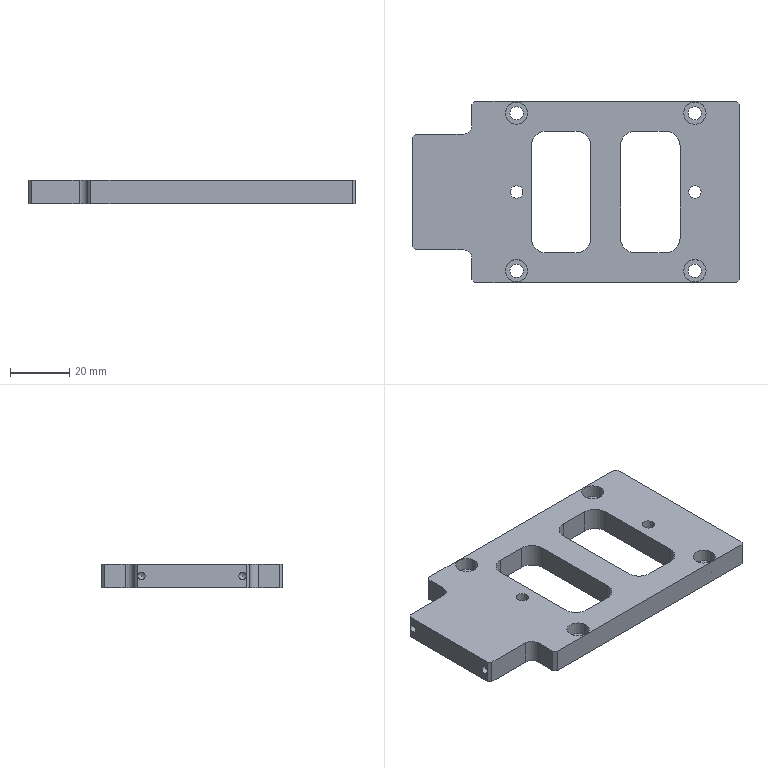Part | 1 solid | 56 faces | box 110 x 61 x 8 mm | volume 35951 mm3 | plane 28 | cylinder 24 | cone 4 | commonest cylinder face diameters 10 x8 2.5 x4 4.5 x4 7.5 x4 4.2 x2 6 x2
STEP:
#1=CARTESIAN_POINT('',(35.,-15.5,4.));
#2=VERTEX_POINT('',#1);
#3=CARTESIAN_POINT('',(35.,15.5,4.));
#4=VERTEX_POINT('',#3);
#5=CARTESIAN_POINT('',(35.,-15.5,4.));
#6=DIRECTION('',(0.,1.,0.));
#7=VECTOR('',#6,1000.);
#8=LINE('',#5,#7);
#9=EDGE_CURVE('',#2,#4,#8,.T.);
#10=ORIENTED_EDGE('',*,*,#9,.T.);
#11=CARTESIAN_POINT('',(35.,15.5,-4.));
#12=VERTEX_POINT('',#11);
#13=CARTESIAN_POINT('',(35.,15.5,-4.));
#14=DIRECTION('',(0.,0.,1.));
#15=VECTOR('',#14,1000.);
#16=LINE('',#13,#15);
#17=EDGE_CURVE('',#12,#4,#16,.T.);
#18=ORIENTED_EDGE('',*,*,#17,.F.);
#19=CARTESIAN_POINT('',(35.,-15.5,-4.));
#20=VERTEX_POINT('',#19);
#21=CARTESIAN_POINT('',(35.,-15.5,-4.));
#22=DIRECTION('',(0.,1.,0.));
#23=VECTOR('',#22,1000.);
#24=LINE('',#21,#23);
#25=EDGE_CURVE('',#20,#12,#24,.T.);
#26=ORIENTED_EDGE('',*,*,#25,.F.);
#27=CARTESIAN_POINT('',(35.,-15.5,-4.));
#28=DIRECTION('',(0.,0.,1.));
#29=VECTOR('',#28,1000.);
#30=LINE('',#27,#29);
#31=EDGE_CURVE('',#20,#2,#30,.T.);
#32=ORIENTED_EDGE('',*,*,#31,.T.);
#33=EDGE_LOOP('',(#10,#18,#26,#32));
#34=FACE_BOUND('',#33,.T.);
#35=CARTESIAN_POINT('',(35.,-15.5,-4.));
#36=DIRECTION('',(1.,0.,0.));
#37=DIRECTION('',(0.,0.,-1.));
#38=AXIS2_PLACEMENT_3D('',#35,#36,#37);
#39=PLANE('',#38);
#40=ADVANCED_FACE('',(#34),#39,.F.);
#41=CARTESIAN_POINT('',(30.,20.5,4.));
#42=VERTEX_POINT('',#41);
#43=CARTESIAN_POINT('',(30.,15.5,4.));
#44=DIRECTION('',(0.,0.,1.));
#45=DIRECTION('',(-1.,0.,0.));
#46=AXIS2_PLACEMENT_3D('',#43,#44,#45);
#47=CIRCLE('',#46,5.);
#48=EDGE_CURVE('',#4,#42,#47,.T.);
#49=ORIENTED_EDGE('',*,*,#48,.T.);
#50=CARTESIAN_POINT('',(30.,20.5,-4.));
#51=VERTEX_POINT('',#50);
#52=CARTESIAN_POINT('',(30.,20.5,-4.));
#53=DIRECTION('',(0.,0.,1.));
#54=VECTOR('',#53,1000.);
#55=LINE('',#52,#54);
#56=EDGE_CURVE('',#51,#42,#55,.T.);
#57=ORIENTED_EDGE('',*,*,#56,.F.);
#58=CARTESIAN_POINT('',(30.,15.5,-4.));
#59=DIRECTION('',(0.,0.,1.));
#60=DIRECTION('',(-1.,0.,0.));
#61=AXIS2_PLACEMENT_3D('',#58,#59,#60);
#62=CIRCLE('',#61,5.);
#63=EDGE_CURVE('',#12,#51,#62,.T.);
#64=ORIENTED_EDGE('',*,*,#63,.F.);
#65=ORIENTED_EDGE('',*,*,#17,.T.);
#66=EDGE_LOOP('',(#49,#57,#64,#65));
#67=FACE_BOUND('',#66,.T.);
#68=CARTESIAN_POINT('',(30.,15.5,-4.));
#69=DIRECTION('',(0.,0.,1.));
#70=DIRECTION('',(1.,0.,0.));
#71=AXIS2_PLACEMENT_3D('',#68,#69,#70);
#72=CYLINDRICAL_SURFACE('',#71,5.);
#73=ADVANCED_FACE('',(#67),#72,.F.);
#74=CARTESIAN_POINT('',(20.,20.5,4.));
#75=VERTEX_POINT('',#74);
#76=CARTESIAN_POINT('',(20.,20.5,4.));
#77=DIRECTION('',(-1.,0.,0.));
#78=VECTOR('',#77,1000.);
#79=LINE('',#76,#78);
#80=EDGE_CURVE('',#42,#75,#79,.T.);
#81=ORIENTED_EDGE('',*,*,#80,.T.);
#82=CARTESIAN_POINT('',(20.,20.5,-4.));
#83=VERTEX_POINT('',#82);
#84=CARTESIAN_POINT('',(20.,20.5,-4.));
#85=DIRECTION('',(0.,0.,1.));
#86=VECTOR('',#85,1000.);
#87=LINE('',#84,#86);
#88=EDGE_CURVE('',#83,#75,#87,.T.);
#89=ORIENTED_EDGE('',*,*,#88,.F.);
#90=CARTESIAN_POINT('',(20.,20.5,-4.));
#91=DIRECTION('',(-1.,0.,0.));
#92=VECTOR('',#91,1000.);
#93=LINE('',#90,#92);
#94=EDGE_CURVE('',#51,#83,#93,.T.);
#95=ORIENTED_EDGE('',*,*,#94,.F.);
#96=ORIENTED_EDGE('',*,*,#56,.T.);
#97=EDGE_LOOP('',(#81,#89,#95,#96));
#98=FACE_BOUND('',#97,.T.);
#99=CARTESIAN_POINT('',(20.,20.5,-4.));
#100=DIRECTION('',(0.,1.,0.));
#101=DIRECTION('',(-1.,0.,0.));
#102=AXIS2_PLACEMENT_3D('',#99,#100,#101);
#103=PLANE('',#102);
#104=ADVANCED_FACE('',(#98),#103,.F.);
#105=CARTESIAN_POINT('',(15.,15.5,4.));
#106=VERTEX_POINT('',#105);
#107=CARTESIAN_POINT('',(20.,15.5,4.));
#108=DIRECTION('',(0.,0.,1.));
#109=DIRECTION('',(-1.,0.,0.));
#110=AXIS2_PLACEMENT_3D('',#107,#108,#109);
#111=CIRCLE('',#110,5.);
#112=EDGE_CURVE('',#75,#106,#111,.T.);
#113=ORIENTED_EDGE('',*,*,#112,.T.);
#114=CARTESIAN_POINT('',(15.,15.5,-4.));
#115=VERTEX_POINT('',#114);
#116=CARTESIAN_POINT('',(15.,15.5,-4.));
#117=DIRECTION('',(0.,0.,1.));
#118=VECTOR('',#117,1000.);
#119=LINE('',#116,#118);
#120=EDGE_CURVE('',#115,#106,#119,.T.);
#121=ORIENTED_EDGE('',*,*,#120,.F.);
#122=CARTESIAN_POINT('',(20.,15.5,-4.));
#123=DIRECTION('',(0.,0.,1.));
#124=DIRECTION('',(-1.,0.,0.));
#125=AXIS2_PLACEMENT_3D('',#122,#123,#124);
#126=CIRCLE('',#125,5.);
#127=EDGE_CURVE('',#83,#115,#126,.T.);
#128=ORIENTED_EDGE('',*,*,#127,.F.);
#129=ORIENTED_EDGE('',*,*,#88,.T.);
#130=EDGE_LOOP('',(#113,#121,#128,#129));
#131=FACE_BOUND('',#130,.T.);
#132=CARTESIAN_POINT('',(20.,15.5,-4.));
#133=DIRECTION('',(0.,0.,1.));
#134=DIRECTION('',(1.,0.,0.));
#135=AXIS2_PLACEMENT_3D('',#132,#133,#134);
#136=CYLINDRICAL_SURFACE('',#135,5.);
#137=ADVANCED_FACE('',(#131),#136,.F.);
#138=CARTESIAN_POINT('',(15.,-15.5,4.));
#139=VERTEX_POINT('',#138);
#140=CARTESIAN_POINT('',(15.,-15.5,4.));
#141=DIRECTION('',(0.,-1.,0.));
#142=VECTOR('',#141,1000.);
#143=LINE('',#140,#142);
#144=EDGE_CURVE('',#106,#139,#143,.T.);
#145=ORIENTED_EDGE('',*,*,#144,.T.);
#146=CARTESIAN_POINT('',(15.,-15.5,-4.));
#147=VERTEX_POINT('',#146);
#148=CARTESIAN_POINT('',(15.,-15.5,-4.));
#149=DIRECTION('',(0.,0.,1.));
#150=VECTOR('',#149,1000.);
#151=LINE('',#148,#150);
#152=EDGE_CURVE('',#147,#139,#151,.T.);
#153=ORIENTED_EDGE('',*,*,#152,.F.);
#154=CARTESIAN_POINT('',(15.,-15.5,-4.));
#155=DIRECTION('',(0.,-1.,0.));
#156=VECTOR('',#155,1000.);
#157=LINE('',#154,#156);
#158=EDGE_CURVE('',#115,#147,#157,.T.);
#159=ORIENTED_EDGE('',*,*,#158,.F.);
#160=ORIENTED_EDGE('',*,*,#120,.T.);
#161=EDGE_LOOP('',(#145,#153,#159,#160));
#162=FACE_BOUND('',#161,.T.);
#163=CARTESIAN_POINT('',(15.,-15.5,-4.));
#164=DIRECTION('',(-1.,0.,0.));
#165=DIRECTION('',(0.,0.,1.));
#166=AXIS2_PLACEMENT_3D('',#163,#164,#165);
#167=PLANE('',#166);
#168=ADVANCED_FACE('',(#162),#167,.F.);
#169=CARTESIAN_POINT('',(20.,-20.5,4.));
#170=VERTEX_POINT('',#169);
#171=CARTESIAN_POINT('',(20.,-15.5,4.));
#172=DIRECTION('',(0.,0.,1.));
#173=DIRECTION('',(-1.,0.,0.));
#174=AXIS2_PLACEMENT_3D('',#171,#172,#173);
#175=CIRCLE('',#174,5.);
#176=EDGE_CURVE('',#139,#170,#175,.T.);
#177=ORIENTED_EDGE('',*,*,#176,.T.);
#178=CARTESIAN_POINT('',(20.,-20.5,-4.));
#179=VERTEX_POINT('',#178);
#180=CARTESIAN_POINT('',(20.,-20.5,-4.));
#181=DIRECTION('',(0.,0.,1.));
#182=VECTOR('',#181,1000.);
#183=LINE('',#180,#182);
#184=EDGE_CURVE('',#179,#170,#183,.T.);
#185=ORIENTED_EDGE('',*,*,#184,.F.);
#186=CARTESIAN_POINT('',(20.,-15.5,-4.));
#187=DIRECTION('',(0.,0.,1.));
#188=DIRECTION('',(-1.,0.,0.));
#189=AXIS2_PLACEMENT_3D('',#186,#187,#188);
#190=CIRCLE('',#189,5.);
#191=EDGE_CURVE('',#147,#179,#190,.T.);
#192=ORIENTED_EDGE('',*,*,#191,.F.);
#193=ORIENTED_EDGE('',*,*,#152,.T.);
#194=EDGE_LOOP('',(#177,#185,#192,#193));
#195=FACE_BOUND('',#194,.T.);
#196=CARTESIAN_POINT('',(20.,-15.5,-4.));
#197=DIRECTION('',(0.,0.,1.));
#198=DIRECTION('',(1.,0.,0.));
#199=AXIS2_PLACEMENT_3D('',#196,#197,#198);
#200=CYLINDRICAL_SURFACE('',#199,5.);
#201=ADVANCED_FACE('',(#195),#200,.F.);
#202=CARTESIAN_POINT('',(30.,-20.5,4.));
#203=VERTEX_POINT('',#202);
#204=CARTESIAN_POINT('',(0.,-20.5,4.));
#205=DIRECTION('',(1.,0.,0.));
#206=VECTOR('',#205,1000.);
#207=LINE('',#204,#206);
#208=EDGE_CURVE('',#170,#203,#207,.T.);
#209=ORIENTED_EDGE('',*,*,#208,.T.);
#210=CARTESIAN_POINT('',(30.,-20.5,-4.));
#211=VERTEX_POINT('',#210);
#212=CARTESIAN_POINT('',(30.,-20.5,-4.));
#213=DIRECTION('',(0.,0.,1.));
#214=VECTOR('',#213,1000.);
#215=LINE('',#212,#214);
#216=EDGE_CURVE('',#211,#203,#215,.T.);
#217=ORIENTED_EDGE('',*,*,#216,.F.);
#218=CARTESIAN_POINT('',(0.,-20.5,-4.));
#219=DIRECTION('',(1.,0.,0.));
#220=VECTOR('',#219,1000.);
#221=LINE('',#218,#220);
#222=EDGE_CURVE('',#179,#211,#221,.T.);
#223=ORIENTED_EDGE('',*,*,#222,.F.);
#224=ORIENTED_EDGE('',*,*,#184,.T.);
#225=EDGE_LOOP('',(#209,#217,#223,#224));
#226=FACE_BOUND('',#225,.T.);
#227=CARTESIAN_POINT('',(0.,-20.5,-4.));
#228=DIRECTION('',(0.,-1.,0.));
#229=DIRECTION('',(0.,0.,-1.));
#230=AXIS2_PLACEMENT_3D('',#227,#228,#229);
#231=PLANE('',#230);
#232=ADVANCED_FACE('',(#226),#231,.F.);
#233=CARTESIAN_POINT('',(30.,-15.5,4.));
#234=DIRECTION('',(0.,0.,1.));
#235=DIRECTION('',(1.,0.,0.));
#236=AXIS2_PLACEMENT_3D('',#233,#234,#235);
#237=CIRCLE('',#236,5.);
#238=EDGE_CURVE('',#203,#2,#237,.T.);
#239=ORIENTED_EDGE('',*,*,#238,.T.);
#240=ORIENTED_EDGE('',*,*,#31,.F.);
#241=CARTESIAN_POINT('',(30.,-15.5,-4.));
#242=DIRECTION('',(0.,0.,1.));
#243=DIRECTION('',(1.,0.,0.));
#244=AXIS2_PLACEMENT_3D('',#241,#242,#243);
#245=CIRCLE('',#244,5.);
#246=EDGE_CURVE('',#211,#20,#245,.T.);
#247=ORIENTED_EDGE('',*,*,#246,.F.);
#248=ORIENTED_EDGE('',*,*,#216,.T.);
#249=EDGE_LOOP('',(#239,#240,#247,#248));
#250=FACE_BOUND('',#249,.T.);
#251=CARTESIAN_POINT('',(30.,-15.5,-4.));
#252=DIRECTION('',(0.,0.,1.));
#253=DIRECTION('',(1.,0.,0.));
#254=AXIS2_PLACEMENT_3D('',#251,#252,#253);
#255=CYLINDRICAL_SURFACE('',#254,5.);
#256=ADVANCED_FACE('',(#250),#255,.F.);
#257=CARTESIAN_POINT('',(0.,20.5,4.));
#258=VERTEX_POINT('',#257);
#259=CARTESIAN_POINT('',(-10.,20.5,4.));
#260=VERTEX_POINT('',#259);
#261=CARTESIAN_POINT('',(20.,20.5,4.));
#262=DIRECTION('',(-1.,0.,0.));
#263=VECTOR('',#262,1000.);
#264=LINE('',#261,#263);
#265=EDGE_CURVE('',#258,#260,#264,.T.);
#266=ORIENTED_EDGE('',*,*,#265,.T.);
#267=CARTESIAN_POINT('',(-10.,20.5,-4.));
#268=VERTEX_POINT('',#267);
#269=CARTESIAN_POINT('',(-10.,20.5,-4.));
#270=DIRECTION('',(0.,0.,1.));
#271=VECTOR('',#270,1000.);
#272=LINE('',#269,#271);
#273=EDGE_CURVE('',#268,#260,#272,.T.);
#274=ORIENTED_EDGE('',*,*,#273,.F.);
#275=CARTESIAN_POINT('',(0.,20.5,-4.));
#276=VERTEX_POINT('',#275);
#277=CARTESIAN_POINT('',(0.,20.5,-4.));
#278=DIRECTION('',(-1.,0.,0.));
#279=VECTOR('',#278,1000.);
#280=LINE('',#277,#279);
#281=EDGE_CURVE('',#276,#268,#280,.T.);
#282=ORIENTED_EDGE('',*,*,#281,.F.);
#283=CARTESIAN_POINT('',(0.,20.5,-4.));
#284=DIRECTION('',(0.,0.,1.));
#285=VECTOR('',#284,1000.);
#286=LINE('',#283,#285);
#287=EDGE_CURVE('',#276,#258,#286,.T.);
#288=ORIENTED_EDGE('',*,*,#287,.T.);
#289=EDGE_LOOP('',(#266,#274,#282,#288));
#290=FACE_BOUND('',#289,.T.);
#291=CARTESIAN_POINT('',(20.,20.5,-4.));
#292=DIRECTION('',(0.,1.,0.));
#293=DIRECTION('',(-1.,0.,0.));
#294=AXIS2_PLACEMENT_3D('',#291,#292,#293);
#295=PLANE('',#294);
#296=ADVANCED_FACE('',(#290),#295,.F.);
#297=CARTESIAN_POINT('',(-15.,15.5,4.));
#298=VERTEX_POINT('',#297);
#299=CARTESIAN_POINT('',(-10.,15.5,4.));
#300=DIRECTION('',(0.,0.,1.));
#301=DIRECTION('',(1.,0.,0.));
#302=AXIS2_PLACEMENT_3D('',#299,#300,#301);
#303=CIRCLE('',#302,5.);
#304=EDGE_CURVE('',#260,#298,#303,.T.);
#305=ORIENTED_EDGE('',*,*,#304,.T.);
#306=CARTESIAN_POINT('',(-15.,15.5,-4.));
#307=VERTEX_POINT('',#306);
#308=CARTESIAN_POINT('',(-15.,15.5,-4.));
#309=DIRECTION('',(0.,0.,1.));
#310=VECTOR('',#309,1000.);
#311=LINE('',#308,#310);
#312=EDGE_CURVE('',#307,#298,#311,.T.);
#313=ORIENTED_EDGE('',*,*,#312,.F.);
#314=CARTESIAN_POINT('',(-10.,15.5,-4.));
#315=DIRECTION('',(0.,0.,1.));
#316=DIRECTION('',(1.,0.,0.));
#317=AXIS2_PLACEMENT_3D('',#314,#315,#316);
#318=CIRCLE('',#317,5.);
#319=EDGE_CURVE('',#268,#307,#318,.T.);
#320=ORIENTED_EDGE('',*,*,#319,.F.);
#321=ORIENTED_EDGE('',*,*,#273,.T.);
#322=EDGE_LOOP('',(#305,#313,#320,#321));
#323=FACE_BOUND('',#322,.T.);
#324=CARTESIAN_POINT('',(-10.,15.5,-4.));
#325=DIRECTION('',(0.,0.,1.));
#326=DIRECTION('',(1.,0.,0.));
#327=AXIS2_PLACEMENT_3D('',#324,#325,#326);
#328=CYLINDRICAL_SURFACE('',#327,5.);
#329=ADVANCED_FACE('',(#323),#328,.F.);
#330=CARTESIAN_POINT('',(-15.,-15.5,4.));
#331=VERTEX_POINT('',#330);
#332=CARTESIAN_POINT('',(-15.,-15.5,4.));
#333=DIRECTION('',(0.,-1.,0.));
#334=VECTOR('',#333,1000.);
#335=LINE('',#332,#334);
#336=EDGE_CURVE('',#298,#331,#335,.T.);
#337=ORIENTED_EDGE('',*,*,#336,.T.);
#338=CARTESIAN_POINT('',(-15.,-15.5,-4.));
#339=VERTEX_POINT('',#338);
#340=CARTESIAN_POINT('',(-15.,-15.5,-4.));
#341=DIRECTION('',(0.,0.,1.));
#342=VECTOR('',#341,1000.);
#343=LINE('',#340,#342);
#344=EDGE_CURVE('',#339,#331,#343,.T.);
#345=ORIENTED_EDGE('',*,*,#344,.F.);
#346=CARTESIAN_POINT('',(-15.,-15.5,-4.));
#347=DIRECTION('',(0.,-1.,0.));
#348=VECTOR('',#347,1000.);
#349=LINE('',#346,#348);
#350=EDGE_CURVE('',#307,#339,#349,.T.);
#351=ORIENTED_EDGE('',*,*,#350,.F.);
#352=ORIENTED_EDGE('',*,*,#312,.T.);
#353=EDGE_LOOP('',(#337,#345,#351,#352));
#354=FACE_BOUND('',#353,.T.);
#355=CARTESIAN_POINT('',(-15.,-15.5,-4.));
#356=DIRECTION('',(-1.,0.,0.));
#357=DIRECTION('',(0.,-1.,0.));
#358=AXIS2_PLACEMENT_3D('',#355,#356,#357);
#359=PLANE('',#358);
#360=ADVANCED_FACE('',(#354),#359,.F.);
#361=CARTESIAN_POINT('',(-10.,-20.5,4.));
#362=VERTEX_POINT('',#361);
#363=CARTESIAN_POINT('',(-10.,-15.5,4.));
#364=DIRECTION('',(0.,0.,1.));
#365=DIRECTION('',(-1.,0.,0.));
#366=AXIS2_PLACEMENT_3D('',#363,#364,#365);
#367=CIRCLE('',#366,5.);
#368=EDGE_CURVE('',#331,#362,#367,.T.);
#369=ORIENTED_EDGE('',*,*,#368,.T.);
#370=CARTESIAN_POINT('',(-10.,-20.5,-4.));
#371=VERTEX_POINT('',#370);
#372=CARTESIAN_POINT('',(-10.,-20.5,-4.));
#373=DIRECTION('',(0.,0.,1.));
#374=VECTOR('',#373,1000.);
#375=LINE('',#372,#374);
#376=EDGE_CURVE('',#371,#362,#375,.T.);
#377=ORIENTED_EDGE('',*,*,#376,.F.);
#378=CARTESIAN_POINT('',(-10.,-15.5,-4.));
#379=DIRECTION('',(0.,0.,1.));
#380=DIRECTION('',(-1.,0.,0.));
#381=AXIS2_PLACEMENT_3D('',#378,#379,#380);
#382=CIRCLE('',#381,5.);
#383=EDGE_CURVE('',#339,#371,#382,.T.);
#384=ORIENTED_EDGE('',*,*,#383,.F.);
#385=ORIENTED_EDGE('',*,*,#344,.T.);
#386=EDGE_LOOP('',(#369,#377,#384,#385));
#387=FACE_BOUND('',#386,.T.);
#388=CARTESIAN_POINT('',(-10.,-15.5,-4.));
#389=DIRECTION('',(0.,0.,1.));
#390=DIRECTION('',(1.,0.,0.));
#391=AXIS2_PLACEMENT_3D('',#388,#389,#390);
#392=CYLINDRICAL_SURFACE('',#391,5.);
#393=ADVANCED_FACE('',(#387),#392,.F.);
#394=CARTESIAN_POINT('',(0.,-20.5,4.));
#395=VERTEX_POINT('',#394);
#396=CARTESIAN_POINT('',(0.,-20.5,4.));
#397=DIRECTION('',(1.,0.,0.));
#398=VECTOR('',#397,1000.);
#399=LINE('',#396,#398);
#400=EDGE_CURVE('',#362,#395,#399,.T.);
#401=ORIENTED_EDGE('',*,*,#400,.T.);
#402=CARTESIAN_POINT('',(0.,-20.5,-4.));
#403=VERTEX_POINT('',#402);
#404=CARTESIAN_POINT('',(0.,-20.5,-4.));
#405=DIRECTION('',(0.,0.,1.));
#406=VECTOR('',#405,1000.);
#407=LINE('',#404,#406);
#408=EDGE_CURVE('',#403,#395,#407,.T.);
#409=ORIENTED_EDGE('',*,*,#408,.F.);
#410=CARTESIAN_POINT('',(0.,-20.5,-4.));
#411=DIRECTION('',(1.,0.,0.));
#412=VECTOR('',#411,1000.);
#413=LINE('',#410,#412);
#414=EDGE_CURVE('',#371,#403,#413,.T.);
#415=ORIENTED_EDGE('',*,*,#414,.F.);
#416=ORIENTED_EDGE('',*,*,#376,.T.);
#417=EDGE_LOOP('',(#401,#409,#415,#416));
#418=FACE_BOUND('',#417,.T.);
#419=CARTESIAN_POINT('',(0.,-20.5,-4.));
#420=DIRECTION('',(0.,-1.,0.));
#421=DIRECTION('',(0.,0.,-1.));
#422=AXIS2_PLACEMENT_3D('',#419,#420,#421);
#423=PLANE('',#422);
#424=ADVANCED_FACE('',(#418),#423,.F.);
#425=CARTESIAN_POINT('',(5.,-15.5,4.));
#426=VERTEX_POINT('',#425);
#427=CARTESIAN_POINT('',(0.,-15.5,4.));
#428=DIRECTION('',(0.,0.,1.));
#429=DIRECTION('',(1.,0.,0.));
#430=AXIS2_PLACEMENT_3D('',#427,#428,#429);
#431=CIRCLE('',#430,5.);
#432=EDGE_CURVE('',#395,#426,#431,.T.);
#433=ORIENTED_EDGE('',*,*,#432,.T.);
#434=CARTESIAN_POINT('',(5.,-15.5,-4.));
#435=VERTEX_POINT('',#434);
#436=CARTESIAN_POINT('',(5.,-15.5,-4.));
#437=DIRECTION('',(0.,0.,1.));
#438=VECTOR('',#437,1000.);
#439=LINE('',#436,#438);
#440=EDGE_CURVE('',#435,#426,#439,.T.);
#441=ORIENTED_EDGE('',*,*,#440,.F.);
#442=CARTESIAN_POINT('',(0.,-15.5,-4.));
#443=DIRECTION('',(0.,0.,1.));
#444=DIRECTION('',(1.,0.,0.));
#445=AXIS2_PLACEMENT_3D('',#442,#443,#444);
#446=CIRCLE('',#445,5.);
#447=EDGE_CURVE('',#403,#435,#446,.T.);
#448=ORIENTED_EDGE('',*,*,#447,.F.);
#449=ORIENTED_EDGE('',*,*,#408,.T.);
#450=EDGE_LOOP('',(#433,#441,#448,#449));
#451=FACE_BOUND('',#450,.T.);
#452=CARTESIAN_POINT('',(0.,-15.5,-4.));
#453=DIRECTION('',(0.,0.,1.));
#454=DIRECTION('',(1.,0.,0.));
#455=AXIS2_PLACEMENT_3D('',#452,#453,#454);
#456=CYLINDRICAL_SURFACE('',#455,5.);
#457=ADVANCED_FACE('',(#451),#456,.F.);
#458=CARTESIAN_POINT('',(5.,15.5,4.));
#459=VERTEX_POINT('',#458);
#460=CARTESIAN_POINT('',(5.,-15.5,4.));
#461=DIRECTION('',(0.,1.,0.));
#462=VECTOR('',#461,1000.);
#463=LINE('',#460,#462);
#464=EDGE_CURVE('',#426,#459,#463,.T.);
#465=ORIENTED_EDGE('',*,*,#464,.T.);
#466=CARTESIAN_POINT('',(5.,15.5,-4.));
#467=VERTEX_POINT('',#466);
#468=CARTESIAN_POINT('',(5.,15.5,-4.));
#469=DIRECTION('',(0.,0.,1.));
#470=VECTOR('',#469,1000.);
#471=LINE('',#468,#470);
#472=EDGE_CURVE('',#467,#459,#471,.T.);
#473=ORIENTED_EDGE('',*,*,#472,.F.);
#474=CARTESIAN_POINT('',(5.,-15.5,-4.));
#475=DIRECTION('',(0.,1.,0.));
#476=VECTOR('',#475,1000.);
#477=LINE('',#474,#476);
#478=EDGE_CURVE('',#435,#467,#477,.T.);
#479=ORIENTED_EDGE('',*,*,#478,.F.);
#480=ORIENTED_EDGE('',*,*,#440,.T.);
#481=EDGE_LOOP('',(#465,#473,#479,#480));
#482=FACE_BOUND('',#481,.T.);
#483=CARTESIAN_POINT('',(5.,-15.5,-4.));
#484=DIRECTION('',(1.,0.,0.));
#485=DIRECTION('',(0.,1.,0.));
#486=AXIS2_PLACEMENT_3D('',#483,#484,#485);
#487=PLANE('',#486);
#488=ADVANCED_FACE('',(#482),#487,.F.);
#489=CARTESIAN_POINT('',(0.,15.5,4.));
#490=DIRECTION('',(0.,0.,1.));
#491=DIRECTION('',(1.,0.,0.));
#492=AXIS2_PLACEMENT_3D('',#489,#490,#491);
#493=CIRCLE('',#492,5.);
#494=EDGE_CURVE('',#459,#258,#493,.T.);
#495=ORIENTED_EDGE('',*,*,#494,.T.);
#496=ORIENTED_EDGE('',*,*,#287,.F.);
#497=CARTESIAN_POINT('',(0.,15.5,-4.));
#498=DIRECTION('',(0.,0.,1.));
#499=DIRECTION('',(1.,0.,0.));
#500=AXIS2_PLACEMENT_3D('',#497,#498,#499);
#501=CIRCLE('',#500,5.);
#502=EDGE_CURVE('',#467,#276,#501,.T.);
#503=ORIENTED_EDGE('',*,*,#502,.F.);
#504=ORIENTED_EDGE('',*,*,#472,.T.);
#505=EDGE_LOOP('',(#495,#496,#503,#504));
#506=FACE_BOUND('',#505,.T.);
#507=CARTESIAN_POINT('',(0.,15.5,-4.));
#508=DIRECTION('',(0.,0.,1.));
#509=DIRECTION('',(1.,0.,0.));
#510=AXIS2_PLACEMENT_3D('',#507,#508,#509);
#511=CYLINDRICAL_SURFACE('',#510,5.);
#512=ADVANCED_FACE('',(#506),#511,.F.);
#513=CARTESIAN_POINT('',(55.,29.5,4.));
#514=VERTEX_POINT('',#513);
#515=CARTESIAN_POINT('',(54.,30.5,4.));
#516=VERTEX_POINT('',#515);
#517=CARTESIAN_POINT('',(42.25,42.25,4.));
#518=DIRECTION('',(-0.7071,0.7071,0.));
#519=VECTOR('',#518,1000.);
#520=LINE('',#517,#519);
#521=EDGE_CURVE('',#514,#516,#520,.T.);
#522=ORIENTED_EDGE('',*,*,#521,.F.);
#523=CARTESIAN_POINT('',(55.,29.5,-4.));
#524=VERTEX_POINT('',#523);
#525=CARTESIAN_POINT('',(55.,29.5,4.));
#526=DIRECTION('',(0.,0.,1.));
#527=VECTOR('',#526,1000.);
#528=LINE('',#525,#527);
#529=EDGE_CURVE('',#524,#514,#528,.T.);
#530=ORIENTED_EDGE('',*,*,#529,.F.);
#531=CARTESIAN_POINT('',(54.,30.5,-4.));
#532=VERTEX_POINT('',#531);
#533=CARTESIAN_POINT('',(54.,30.5,-4.));
#534=DIRECTION('',(0.7071,-0.7071,0.));
#535=VECTOR('',#534,1000.);
#536=LINE('',#533,#535);
#537=EDGE_CURVE('',#532,#524,#536,.T.);
#538=ORIENTED_EDGE('',*,*,#537,.F.);
#539=CARTESIAN_POINT('',(54.,30.5,4.));
#540=DIRECTION('',(0.,0.,-1.));
#541=VECTOR('',#540,1000.);
#542=LINE('',#539,#541);
#543=EDGE_CURVE('',#516,#532,#542,.T.);
#544=ORIENTED_EDGE('',*,*,#543,.F.);
#545=EDGE_LOOP('',(#522,#530,#538,#544));
#546=FACE_BOUND('',#545,.T.);
#547=CARTESIAN_POINT('',(54.,30.5,4.));
#548=DIRECTION('',(-0.7071,-0.7071,0.));
#549=DIRECTION('',(0.,0.,-1.));
#550=AXIS2_PLACEMENT_3D('',#547,#548,#549);
#551=PLANE('',#550);
#552=ADVANCED_FACE('',(#546),#551,.F.);
#553=CARTESIAN_POINT('',(54.,-30.5,4.));
#554=VERTEX_POINT('',#553);
#555=CARTESIAN_POINT('',(55.,-29.5,4.));
#556=VERTEX_POINT('',#555);
#557=CARTESIAN_POINT('',(42.25,-42.25,4.));
#558=DIRECTION('',(0.7071,0.7071,0.));
#559=VECTOR('',#558,1000.);
#560=LINE('',#557,#559);
#561=EDGE_CURVE('',#554,#556,#560,.T.);
#562=ORIENTED_EDGE('',*,*,#561,.F.);
#563=CARTESIAN_POINT('',(54.,-30.5,-4.));
#564=VERTEX_POINT('',#563);
#565=CARTESIAN_POINT('',(54.,-30.5,4.));
#566=DIRECTION('',(0.,0.,1.));
#567=VECTOR('',#566,1000.);
#568=LINE('',#565,#567);
#569=EDGE_CURVE('',#564,#554,#568,.T.);
#570=ORIENTED_EDGE('',*,*,#569,.F.);
#571=CARTESIAN_POINT('',(55.,-29.5,-4.));
#572=VERTEX_POINT('',#571);
#573=CARTESIAN_POINT('',(55.,-29.5,-4.));
#574=DIRECTION('',(-0.7071,-0.7071,0.));
#575=VECTOR('',#574,1000.);
#576=LINE('',#573,#575);
#577=EDGE_CURVE('',#572,#564,#576,.T.);
#578=ORIENTED_EDGE('',*,*,#577,.F.);
#579=CARTESIAN_POINT('',(55.,-29.5,4.));
#580=DIRECTION('',(0.,0.,-1.));
#581=VECTOR('',#580,1000.);
#582=LINE('',#579,#581);
#583=EDGE_CURVE('',#556,#572,#582,.T.);
#584=ORIENTED_EDGE('',*,*,#583,.F.);
#585=EDGE_LOOP('',(#562,#570,#578,#584));
#586=FACE_BOUND('',#585,.T.);
#587=CARTESIAN_POINT('',(55.,-29.5,4.));
#588=DIRECTION('',(-0.7071,0.7071,0.));
#589=DIRECTION('',(0.,0.,-1.));
#590=AXIS2_PLACEMENT_3D('',#587,#588,#589);
#591=PLANE('',#590);
#592=ADVANCED_FACE('',(#586),#591,.F.);
#593=CARTESIAN_POINT('',(-35.,29.5,-4.));
#594=VERTEX_POINT('',#593);
#595=CARTESIAN_POINT('',(-34.,30.5,-4.));
#596=VERTEX_POINT('',#595);
#597=CARTESIAN_POINT('',(-34.,30.5,-4.));
#598=DIRECTION('',(0.7071,0.7071,0.));
#599=VECTOR('',#598,1000.);
#600=LINE('',#597,#599);
#601=EDGE_CURVE('',#594,#596,#600,.T.);
#602=ORIENTED_EDGE('',*,*,#601,.F.);
#603=CARTESIAN_POINT('',(-35.,29.5,4.));
#604=VERTEX_POINT('',#603);
#605=CARTESIAN_POINT('',(-35.,29.5,-4.));
#606=DIRECTION('',(0.,0.,-1.));
#607=VECTOR('',#606,1000.);
#608=LINE('',#605,#607);
#609=EDGE_CURVE('',#604,#594,#608,.T.);
#610=ORIENTED_EDGE('',*,*,#609,.F.);
#611=CARTESIAN_POINT('',(-34.,30.5,4.));
#612=VERTEX_POINT('',#611);
#613=CARTESIAN_POINT('',(-32.25,32.25,4.));
#614=DIRECTION('',(-0.7071,-0.7071,0.));
#615=VECTOR('',#614,1000.);
#616=LINE('',#613,#615);
#617=EDGE_CURVE('',#612,#604,#616,.T.);
#618=ORIENTED_EDGE('',*,*,#617,.F.);
#619=CARTESIAN_POINT('',(-34.,30.5,4.));
#620=DIRECTION('',(0.,0.,1.));
#621=VECTOR('',#620,1000.);
#622=LINE('',#619,#621);
#623=EDGE_CURVE('',#596,#612,#622,.T.);
#624=ORIENTED_EDGE('',*,*,#623,.F.);
#625=EDGE_LOOP('',(#602,#610,#618,#624));
#626=FACE_BOUND('',#625,.T.);
#627=CARTESIAN_POINT('',(-34.,30.5,4.));
#628=DIRECTION('',(0.7071,-0.7071,0.));
#629=DIRECTION('',(0.,0.,1.));
#630=AXIS2_PLACEMENT_3D('',#627,#628,#629);
#631=PLANE('',#630);
#632=ADVANCED_FACE('',(#626),#631,.F.);
#633=CARTESIAN_POINT('',(-34.,-30.5,-4.));
#634=VERTEX_POINT('',#633);
#635=CARTESIAN_POINT('',(-35.,-29.5,-4.));
#636=VERTEX_POINT('',#635);
#637=CARTESIAN_POINT('',(-35.,-29.5,-4.));
#638=DIRECTION('',(-0.7071,0.7071,0.));
#639=VECTOR('',#638,1000.);
#640=LINE('',#637,#639);
#641=EDGE_CURVE('',#634,#636,#640,.T.);
#642=ORIENTED_EDGE('',*,*,#641,.F.);
#643=CARTESIAN_POINT('',(-34.,-30.5,4.));
#644=VERTEX_POINT('',#643);
#645=CARTESIAN_POINT('',(-34.,-30.5,4.));
#646=DIRECTION('',(0.,0.,-1.));
#647=VECTOR('',#646,1000.);
#648=LINE('',#645,#647);
#649=EDGE_CURVE('',#644,#634,#648,.T.);
#650=ORIENTED_EDGE('',*,*,#649,.F.);
#651=CARTESIAN_POINT('',(-35.,-29.5,4.));
#652=VERTEX_POINT('',#651);
#653=CARTESIAN_POINT('',(-32.25,-32.25,4.));
#654=DIRECTION('',(0.7071,-0.7071,0.));
#655=VECTOR('',#654,1000.);
#656=LINE('',#653,#655);
#657=EDGE_CURVE('',#652,#644,#656,.T.);
#658=ORIENTED_EDGE('',*,*,#657,.F.);
#659=CARTESIAN_POINT('',(-35.,-29.5,-4.));
#660=DIRECTION('',(0.,0.,1.));
#661=VECTOR('',#660,1000.);
#662=LINE('',#659,#661);
#663=EDGE_CURVE('',#636,#652,#662,.T.);
#664=ORIENTED_EDGE('',*,*,#663,.F.);
#665=EDGE_LOOP('',(#642,#650,#658,#664));
#666=FACE_BOUND('',#665,.T.);
#667=CARTESIAN_POINT('',(-35.,-29.5,-4.));
#668=DIRECTION('',(0.7071,0.7071,0.));
#669=DIRECTION('',(0.,0.,1.));
#670=AXIS2_PLACEMENT_3D('',#667,#668,#669);
#671=PLANE('',#670);
#672=ADVANCED_FACE('',(#666),#671,.F.);
#673=CARTESIAN_POINT('',(-55.,18.5,-4.));
#674=VERTEX_POINT('',#673);
#675=CARTESIAN_POINT('',(-54.,19.5,-4.));
#676=VERTEX_POINT('',#675);
#677=CARTESIAN_POINT('',(-54.,19.5,-4.));
#678=DIRECTION('',(0.7071,0.7071,0.));
#679=VECTOR('',#678,1000.);
#680=LINE('',#677,#679);
#681=EDGE_CURVE('',#674,#676,#680,.T.);
#682=ORIENTED_EDGE('',*,*,#681,.F.);
#683=CARTESIAN_POINT('',(-55.,18.5,4.));
#684=VERTEX_POINT('',#683);
#685=CARTESIAN_POINT('',(-55.,18.5,4.));
#686=DIRECTION('',(0.,0.,-1.));
#687=VECTOR('',#686,1000.);
#688=LINE('',#685,#687);
#689=EDGE_CURVE('',#684,#674,#688,.T.);
#690=ORIENTED_EDGE('',*,*,#689,.F.);
#691=CARTESIAN_POINT('',(-54.,19.5,4.));
#692=VERTEX_POINT('',#691);
#693=CARTESIAN_POINT('',(-36.75,36.75,4.));
#694=DIRECTION('',(-0.7071,-0.7071,0.));
#695=VECTOR('',#694,1000.);
#696=LINE('',#693,#695);
#697=EDGE_CURVE('',#692,#684,#696,.T.);
#698=ORIENTED_EDGE('',*,*,#697,.F.);
#699=CARTESIAN_POINT('',(-54.,19.5,-4.));
#700=DIRECTION('',(0.,0.,1.));
#701=VECTOR('',#700,1000.);
#702=LINE('',#699,#701);
#703=EDGE_CURVE('',#676,#692,#702,.T.);
#704=ORIENTED_EDGE('',*,*,#703,.F.);
#705=EDGE_LOOP('',(#682,#690,#698,#704));
#706=FACE_BOUND('',#705,.T.);
#707=CARTESIAN_POINT('',(-54.,19.5,-4.));
#708=DIRECTION('',(0.7071,-0.7071,0.));
#709=DIRECTION('',(0.,0.,1.));
#710=AXIS2_PLACEMENT_3D('',#707,#708,#709);
#711=PLANE('',#710);
#712=ADVANCED_FACE('',(#706),#711,.F.);
#713=CARTESIAN_POINT('',(-54.,-19.5,-4.));
#714=VERTEX_POINT('',#713);
#715=CARTESIAN_POINT('',(-55.,-18.5,-4.));
#716=VERTEX_POINT('',#715);
#717=CARTESIAN_POINT('',(-55.,-18.5,-4.));
#718=DIRECTION('',(-0.7071,0.7071,0.));
#719=VECTOR('',#718,1000.);
#720=LINE('',#717,#719);
#721=EDGE_CURVE('',#714,#716,#720,.T.);
#722=ORIENTED_EDGE('',*,*,#721,.F.);
#723=CARTESIAN_POINT('',(-54.,-19.5,4.));
#724=VERTEX_POINT('',#723);
#725=CARTESIAN_POINT('',(-54.,-19.5,-4.));
#726=DIRECTION('',(0.,0.,-1.));
#727=VECTOR('',#726,1000.);
#728=LINE('',#725,#727);
#729=EDGE_CURVE('',#724,#714,#728,.T.);
#730=ORIENTED_EDGE('',*,*,#729,.F.);
#731=CARTESIAN_POINT('',(-55.,-18.5,4.));
#732=VERTEX_POINT('',#731);
#733=CARTESIAN_POINT('',(-36.75,-36.75,4.));
#734=DIRECTION('',(0.7071,-0.7071,0.));
#735=VECTOR('',#734,1000.);
#736=LINE('',#733,#735);
#737=EDGE_CURVE('',#732,#724,#736,.T.);
#738=ORIENTED_EDGE('',*,*,#737,.F.);
#739=CARTESIAN_POINT('',(-55.,-18.5,4.));
#740=DIRECTION('',(0.,0.,1.));
#741=VECTOR('',#740,1000.);
#742=LINE('',#739,#741);
#743=EDGE_CURVE('',#716,#732,#742,.T.);
#744=ORIENTED_EDGE('',*,*,#743,.F.);
#745=EDGE_LOOP('',(#722,#730,#738,#744));
#746=FACE_BOUND('',#745,.T.);
#747=CARTESIAN_POINT('',(-55.,-18.5,4.));
#748=DIRECTION('',(0.7071,0.7071,0.));
#749=DIRECTION('',(0.,0.,1.));
#750=AXIS2_PLACEMENT_3D('',#747,#748,#749);
#751=PLANE('',#750);
#752=ADVANCED_FACE('',(#746),#751,.F.);
#753=CARTESIAN_POINT('',(-38.,19.5,-4.));
#754=VERTEX_POINT('',#753);
#755=CARTESIAN_POINT('',(-35.,22.5,-4.));
#756=VERTEX_POINT('',#755);
#757=CARTESIAN_POINT('',(-38.,22.5,-4.));
#758=DIRECTION('',(0.,0.,1.));
#759=DIRECTION('',(1.,0.,0.));
#760=AXIS2_PLACEMENT_3D('',#757,#758,#759);
#761=CIRCLE('',#760,3.);
#762=EDGE_CURVE('',#754,#756,#761,.T.);
#763=ORIENTED_EDGE('',*,*,#762,.F.);
#764=CARTESIAN_POINT('',(-38.,19.5,4.));
#765=VERTEX_POINT('',#764);
#766=CARTESIAN_POINT('',(-38.,19.5,-4.));
#767=DIRECTION('',(0.,0.,-1.));
#768=VECTOR('',#767,1000.);
#769=LINE('',#766,#768);
#770=EDGE_CURVE('',#765,#754,#769,.T.);
#771=ORIENTED_EDGE('',*,*,#770,.F.);
#772=CARTESIAN_POINT('',(-35.,22.5,4.));
#773=VERTEX_POINT('',#772);
#774=CARTESIAN_POINT('',(-38.,22.5,4.));
#775=DIRECTION('',(0.,0.,-1.));
#776=DIRECTION('',(1.,0.,0.));
#777=AXIS2_PLACEMENT_3D('',#774,#775,#776);
#778=CIRCLE('',#777,3.);
#779=EDGE_CURVE('',#773,#765,#778,.T.);
#780=ORIENTED_EDGE('',*,*,#779,.F.);
#781=CARTESIAN_POINT('',(-35.,22.5,4.));
#782=DIRECTION('',(0.,0.,1.));
#783=VECTOR('',#782,1000.);
#784=LINE('',#781,#783);
#785=EDGE_CURVE('',#756,#773,#784,.T.);
#786=ORIENTED_EDGE('',*,*,#785,.F.);
#787=EDGE_LOOP('',(#763,#771,#780,#786));
#788=FACE_BOUND('',#787,.T.);
#789=CARTESIAN_POINT('',(-38.,22.5,-4.));
#790=DIRECTION('',(0.,0.,-1.));
#791=DIRECTION('',(-1.,0.,0.));
#792=AXIS2_PLACEMENT_3D('',#789,#790,#791);
#793=CYLINDRICAL_SURFACE('',#792,3.);
#794=ADVANCED_FACE('',(#788),#793,.F.);
#795=CARTESIAN_POINT('',(-35.,-22.5,-4.));
#796=VERTEX_POINT('',#795);
#797=CARTESIAN_POINT('',(-38.,-19.5,-4.));
#798=VERTEX_POINT('',#797);
#799=CARTESIAN_POINT('',(-38.,-22.5,-4.));
#800=DIRECTION('',(0.,0.,1.));
#801=DIRECTION('',(1.,0.,0.));
#802=AXIS2_PLACEMENT_3D('',#799,#800,#801);
#803=CIRCLE('',#802,3.);
#804=EDGE_CURVE('',#796,#798,#803,.T.);
#805=ORIENTED_EDGE('',*,*,#804,.F.);
#806=CARTESIAN_POINT('',(-35.,-22.5,4.));
#807=VERTEX_POINT('',#806);
#808=CARTESIAN_POINT('',(-35.,-22.5,-4.));
#809=DIRECTION('',(0.,0.,-1.));
#810=VECTOR('',#809,1000.);
#811=LINE('',#808,#810);
#812=EDGE_CURVE('',#807,#796,#811,.T.);
#813=ORIENTED_EDGE('',*,*,#812,.F.);
#814=CARTESIAN_POINT('',(-38.,-19.5,4.));
#815=VERTEX_POINT('',#814);
#816=CARTESIAN_POINT('',(-38.,-22.5,4.));
#817=DIRECTION('',(0.,0.,-1.));
#818=DIRECTION('',(1.,0.,0.));
#819=AXIS2_PLACEMENT_3D('',#816,#817,#818);
#820=CIRCLE('',#819,3.);
#821=EDGE_CURVE('',#815,#807,#820,.T.);
#822=ORIENTED_EDGE('',*,*,#821,.F.);
#823=CARTESIAN_POINT('',(-38.,-19.5,4.));
#824=DIRECTION('',(0.,0.,1.));
#825=VECTOR('',#824,1000.);
#826=LINE('',#823,#825);
#827=EDGE_CURVE('',#798,#815,#826,.T.);
#828=ORIENTED_EDGE('',*,*,#827,.F.);
#829=EDGE_LOOP('',(#805,#813,#822,#828));
#830=FACE_BOUND('',#829,.T.);
#831=CARTESIAN_POINT('',(-38.,-22.5,-4.));
#832=DIRECTION('',(0.,0.,-1.));
#833=DIRECTION('',(-1.,0.,0.));
#834=AXIS2_PLACEMENT_3D('',#831,#832,#833);
#835=CYLINDRICAL_SURFACE('',#834,3.);
#836=ADVANCED_FACE('',(#830),#835,.F.);
#837=CARTESIAN_POINT('',(-55.,19.5,-4.));
#838=DIRECTION('',(1.,0.,0.));
#839=VECTOR('',#838,1000.);
#840=LINE('',#837,#839);
#841=EDGE_CURVE('',#676,#754,#840,.T.);
#842=ORIENTED_EDGE('',*,*,#841,.F.);
#843=ORIENTED_EDGE('',*,*,#703,.T.);
#844=CARTESIAN_POINT('',(-55.,19.5,4.));
#845=DIRECTION('',(1.,0.,0.));
#846=VECTOR('',#845,1000.);
#847=LINE('',#844,#846);
#848=EDGE_CURVE('',#692,#765,#847,.T.);
#849=ORIENTED_EDGE('',*,*,#848,.T.);
#850=ORIENTED_EDGE('',*,*,#770,.T.);
#851=EDGE_LOOP('',(#842,#843,#849,#850));
#852=FACE_BOUND('',#851,.T.);
#853=CARTESIAN_POINT('',(-55.,19.5,-4.));
#854=DIRECTION('',(0.,-1.,0.));
#855=DIRECTION('',(0.,0.,-1.));
#856=AXIS2_PLACEMENT_3D('',#853,#854,#855);
#857=PLANE('',#856);
#858=ADVANCED_FACE('',(#852),#857,.F.);
#859=CARTESIAN_POINT('',(-35.,30.5,4.));
#860=DIRECTION('',(0.,1.,0.));
#861=VECTOR('',#860,1000.);
#862=LINE('',#859,#861);
#863=EDGE_CURVE('',#773,#604,#862,.T.);
#864=ORIENTED_EDGE('',*,*,#863,.T.);
#865=ORIENTED_EDGE('',*,*,#609,.T.);
#866=CARTESIAN_POINT('',(-35.,30.5,-4.));
#867=DIRECTION('',(0.,1.,0.));
#868=VECTOR('',#867,1000.);
#869=LINE('',#866,#868);
#870=EDGE_CURVE('',#756,#594,#869,.T.);
#871=ORIENTED_EDGE('',*,*,#870,.F.);
#872=ORIENTED_EDGE('',*,*,#785,.T.);
#873=EDGE_LOOP('',(#864,#865,#871,#872));
#874=FACE_BOUND('',#873,.T.);
#875=CARTESIAN_POINT('',(-35.,30.5,-4.));
#876=DIRECTION('',(1.,0.,0.));
#877=DIRECTION('',(0.,1.,0.));
#878=AXIS2_PLACEMENT_3D('',#875,#876,#877);
#879=PLANE('',#878);
#880=ADVANCED_FACE('',(#874),#879,.F.);
#881=CARTESIAN_POINT('',(-35.,0.,-4.));
#882=DIRECTION('',(0.,1.,0.));
#883=VECTOR('',#882,1000.);
#884=LINE('',#881,#883);
#885=EDGE_CURVE('',#636,#796,#884,.T.);
#886=ORIENTED_EDGE('',*,*,#885,.F.);
#887=ORIENTED_EDGE('',*,*,#663,.T.);
#888=CARTESIAN_POINT('',(-35.,30.5,4.));
#889=DIRECTION('',(0.,1.,0.));
#890=VECTOR('',#889,1000.);
#891=LINE('',#888,#890);
#892=EDGE_CURVE('',#652,#807,#891,.T.);
#893=ORIENTED_EDGE('',*,*,#892,.T.);
#894=ORIENTED_EDGE('',*,*,#812,.T.);
#895=EDGE_LOOP('',(#886,#887,#893,#894));
#896=FACE_BOUND('',#895,.T.);
#897=CARTESIAN_POINT('',(-35.,30.5,-4.));
#898=DIRECTION('',(1.,0.,0.));
#899=DIRECTION('',(0.,1.,0.));
#900=AXIS2_PLACEMENT_3D('',#897,#898,#899);
#901=PLANE('',#900);
#902=ADVANCED_FACE('',(#896),#901,.F.);
#903=CARTESIAN_POINT('',(-55.,-19.5,4.));
#904=DIRECTION('',(-1.,0.,0.));
#905=VECTOR('',#904,1000.);
#906=LINE('',#903,#905);
#907=EDGE_CURVE('',#815,#724,#906,.T.);
#908=ORIENTED_EDGE('',*,*,#907,.T.);
#909=ORIENTED_EDGE('',*,*,#729,.T.);
#910=CARTESIAN_POINT('',(-55.,-19.5,-4.));
#911=DIRECTION('',(-1.,0.,0.));
#912=VECTOR('',#911,1000.);
#913=LINE('',#910,#912);
#914=EDGE_CURVE('',#798,#714,#913,.T.);
#915=ORIENTED_EDGE('',*,*,#914,.F.);
#916=ORIENTED_EDGE('',*,*,#827,.T.);
#917=EDGE_LOOP('',(#908,#909,#915,#916));
#918=FACE_BOUND('',#917,.T.);
#919=CARTESIAN_POINT('',(-55.,-19.5,-4.));
#920=DIRECTION('',(0.,1.,0.));
#921=DIRECTION('',(0.,0.,1.));
#922=AXIS2_PLACEMENT_3D('',#919,#920,#921);
#923=PLANE('',#922);
#924=ADVANCED_FACE('',(#918),#923,.F.);
#925=CARTESIAN_POINT('',(43.75,-26.5,-0.4));
#926=VERTEX_POINT('',#925);
#927=CARTESIAN_POINT('',(40.,-26.5,-0.4));
#928=DIRECTION('',(0.,0.,1.));
#929=DIRECTION('',(1.,0.,0.));
#930=AXIS2_PLACEMENT_3D('',#927,#928,#929);
#931=CIRCLE('',#930,3.75);
#932=EDGE_CURVE('',#926,#926,#931,.T.);
#933=ORIENTED_EDGE('',*,*,#932,.T.);
#934=EDGE_LOOP('',(#933));
#935=FACE_BOUND('',#934,.T.);
#936=CARTESIAN_POINT('',(42.25,-26.5,-0.4));
#937=VERTEX_POINT('',#936);
#938=CARTESIAN_POINT('',(40.,-26.5,-0.4));
#939=DIRECTION('',(0.,0.,1.));
#940=DIRECTION('',(1.,0.,0.));
#941=AXIS2_PLACEMENT_3D('',#938,#939,#940);
#942=CIRCLE('',#941,2.25);
#943=EDGE_CURVE('',#937,#937,#942,.T.);
#944=ORIENTED_EDGE('',*,*,#943,.F.);
#945=EDGE_LOOP('',(#944));
#946=FACE_BOUND('',#945,.T.);
#947=CARTESIAN_POINT('',(42.25,-26.5,-0.4));
#948=DIRECTION('',(0.,0.,-1.));
#949=DIRECTION('',(-1.,0.,0.));
#950=AXIS2_PLACEMENT_3D('',#947,#948,#949);
#951=PLANE('',#950);
#952=ADVANCED_FACE('',(#935,#946),#951,.F.);
#953=CARTESIAN_POINT('',(-23.75,-26.5,-0.4));
#954=VERTEX_POINT('',#953);
#955=CARTESIAN_POINT('',(-20.,-26.5,-0.4));
#956=DIRECTION('',(0.,0.,1.));
#957=DIRECTION('',(-1.,0.,0.));
#958=AXIS2_PLACEMENT_3D('',#955,#956,#957);
#959=CIRCLE('',#958,3.75);
#960=EDGE_CURVE('',#954,#954,#959,.T.);
#961=ORIENTED_EDGE('',*,*,#960,.T.);
#962=EDGE_LOOP('',(#961));
#963=FACE_BOUND('',#962,.T.);
#964=CARTESIAN_POINT('',(-22.25,-26.5,-0.4));
#965=VERTEX_POINT('',#964);
#966=CARTESIAN_POINT('',(-20.,-26.5,-0.4));
#967=DIRECTION('',(0.,0.,1.));
#968=DIRECTION('',(-1.,0.,0.));
#969=AXIS2_PLACEMENT_3D('',#966,#967,#968);
#970=CIRCLE('',#969,2.25);
#971=EDGE_CURVE('',#965,#965,#970,.T.);
#972=ORIENTED_EDGE('',*,*,#971,.F.);
#973=EDGE_LOOP('',(#972));
#974=FACE_BOUND('',#973,.T.);
#975=CARTESIAN_POINT('',(42.25,-26.5,-0.4));
#976=DIRECTION('',(0.,0.,-1.));
#977=DIRECTION('',(-1.,0.,0.));
#978=AXIS2_PLACEMENT_3D('',#975,#976,#977);
#979=PLANE('',#978);
#980=ADVANCED_FACE('',(#963,#974),#979,.F.);
#981=CARTESIAN_POINT('',(-23.75,26.5,-0.4));
#982=VERTEX_POINT('',#981);
#983=CARTESIAN_POINT('',(-20.,26.5,-0.4));
#984=DIRECTION('',(0.,0.,1.));
#985=DIRECTION('',(-1.,0.,0.));
#986=AXIS2_PLACEMENT_3D('',#983,#984,#985);
#987=CIRCLE('',#986,3.75);
#988=EDGE_CURVE('',#982,#982,#987,.T.);
#989=ORIENTED_EDGE('',*,*,#988,.T.);
#990=EDGE_LOOP('',(#989));
#991=FACE_BOUND('',#990,.T.);
#992=CARTESIAN_POINT('',(-22.25,26.5,-0.4));
#993=VERTEX_POINT('',#992);
#994=CARTESIAN_POINT('',(-20.,26.5,-0.4));
#995=DIRECTION('',(0.,0.,1.));
#996=DIRECTION('',(-1.,0.,0.));
#997=AXIS2_PLACEMENT_3D('',#994,#995,#996);
#998=CIRCLE('',#997,2.25);
#999=EDGE_CURVE('',#993,#993,#998,.T.);
#1000=ORIENTED_EDGE('',*,*,#999,.F.);
#1001=EDGE_LOOP('',(#1000));
#1002=FACE_BOUND('',#1001,.T.);
#1003=CARTESIAN_POINT('',(42.25,-26.5,-0.4));
#1004=DIRECTION('',(0.,0.,-1.));
#1005=DIRECTION('',(-1.,0.,0.));
#1006=AXIS2_PLACEMENT_3D('',#1003,#1004,#1005);
#1007=PLANE('',#1006);
#1008=ADVANCED_FACE('',(#991,#1002),#1007,.F.);
#1009=CARTESIAN_POINT('',(36.25,26.5,-0.4));
#1010=VERTEX_POINT('',#1009);
#1011=CARTESIAN_POINT('',(40.,26.5,-0.4));
#1012=DIRECTION('',(0.,0.,1.));
#1013=DIRECTION('',(-1.,0.,0.));
#1014=AXIS2_PLACEMENT_3D('',#1011,#1012,#1013);
#1015=CIRCLE('',#1014,3.75);
#1016=EDGE_CURVE('',#1010,#1010,#1015,.T.);
#1017=ORIENTED_EDGE('',*,*,#1016,.T.);
#1018=EDGE_LOOP('',(#1017));
#1019=FACE_BOUND('',#1018,.T.);
#1020=CARTESIAN_POINT('',(37.75,26.5,-0.4));
#1021=VERTEX_POINT('',#1020);
#1022=CARTESIAN_POINT('',(40.,26.5,-0.4));
#1023=DIRECTION('',(0.,0.,1.));
#1024=DIRECTION('',(-1.,0.,0.));
#1025=AXIS2_PLACEMENT_3D('',#1022,#1023,#1024);
#1026=CIRCLE('',#1025,2.25);
#1027=EDGE_CURVE('',#1021,#1021,#1026,.T.);
#1028=ORIENTED_EDGE('',*,*,#1027,.F.);
#1029=EDGE_LOOP('',(#1028));
#1030=FACE_BOUND('',#1029,.T.);
#1031=CARTESIAN_POINT('',(42.25,-26.5,-0.4));
#1032=DIRECTION('',(0.,0.,-1.));
#1033=DIRECTION('',(-1.,0.,0.));
#1034=AXIS2_PLACEMENT_3D('',#1031,#1032,#1033);
#1035=PLANE('',#1034);
#1036=ADVANCED_FACE('',(#1019,#1030),#1035,.F.);
#1037=ORIENTED_EDGE('',*,*,#914,.T.);
#1038=ORIENTED_EDGE('',*,*,#721,.T.);
#1039=CARTESIAN_POINT('',(-55.,30.5,-4.));
#1040=DIRECTION('',(0.,-1.,0.));
#1041=VECTOR('',#1040,1000.);
#1042=LINE('',#1039,#1041);
#1043=EDGE_CURVE('',#674,#716,#1042,.T.);
#1044=ORIENTED_EDGE('',*,*,#1043,.F.);
#1045=ORIENTED_EDGE('',*,*,#681,.T.);
#1046=ORIENTED_EDGE('',*,*,#841,.T.);
#1047=ORIENTED_EDGE('',*,*,#762,.T.);
#1048=ORIENTED_EDGE('',*,*,#870,.T.);
#1049=ORIENTED_EDGE('',*,*,#601,.T.);
#1050=CARTESIAN_POINT('',(-55.,30.5,-4.));
#1051=DIRECTION('',(-1.,0.,0.));
#1052=VECTOR('',#1051,1000.);
#1053=LINE('',#1050,#1052);
#1054=EDGE_CURVE('',#532,#596,#1053,.T.);
#1055=ORIENTED_EDGE('',*,*,#1054,.F.);
#1056=ORIENTED_EDGE('',*,*,#537,.T.);
#1057=CARTESIAN_POINT('',(55.,30.5,-4.));
#1058=DIRECTION('',(0.,1.,0.));
#1059=VECTOR('',#1058,1000.);
#1060=LINE('',#1057,#1059);
#1061=EDGE_CURVE('',#572,#524,#1060,.T.);
#1062=ORIENTED_EDGE('',*,*,#1061,.F.);
#1063=ORIENTED_EDGE('',*,*,#577,.T.);
#1064=CARTESIAN_POINT('',(-55.,-30.5,-4.));
#1065=DIRECTION('',(1.,0.,0.));
#1066=VECTOR('',#1065,1000.);
#1067=LINE('',#1064,#1066);
#1068=EDGE_CURVE('',#634,#564,#1067,.T.);
#1069=ORIENTED_EDGE('',*,*,#1068,.F.);
#1070=ORIENTED_EDGE('',*,*,#641,.T.);
#1071=ORIENTED_EDGE('',*,*,#885,.T.);
#1072=ORIENTED_EDGE('',*,*,#804,.T.);
#1073=EDGE_LOOP('',(#1037,#1038,#1044,#1045,#1046,#1047,#1048,#1049,#1055,#1056,#1062,#1063,#1069,#1070,#1071,#1072));
#1074=FACE_BOUND('',#1073,.T.);
#1075=CARTESIAN_POINT('',(42.25,26.5,-4.));
#1076=VERTEX_POINT('',#1075);
#1077=CARTESIAN_POINT('',(40.,26.5,-4.));
#1078=DIRECTION('',(0.,0.,1.));
#1079=DIRECTION('',(1.,0.,0.));
#1080=AXIS2_PLACEMENT_3D('',#1077,#1078,#1079);
#1081=CIRCLE('',#1080,2.25);
#1082=EDGE_CURVE('',#1076,#1076,#1081,.T.);
#1083=ORIENTED_EDGE('',*,*,#1082,.T.);
#1084=EDGE_LOOP('',(#1083));
#1085=FACE_BOUND('',#1084,.T.);
#1086=CARTESIAN_POINT('',(-17.75,26.5,-4.));
#1087=VERTEX_POINT('',#1086);
#1088=CARTESIAN_POINT('',(-20.,26.5,-4.));
#1089=DIRECTION('',(0.,0.,1.));
#1090=DIRECTION('',(1.,0.,0.));
#1091=AXIS2_PLACEMENT_3D('',#1088,#1089,#1090);
#1092=CIRCLE('',#1091,2.25);
#1093=EDGE_CURVE('',#1087,#1087,#1092,.T.);
#1094=ORIENTED_EDGE('',*,*,#1093,.T.);
#1095=EDGE_LOOP('',(#1094));
#1096=FACE_BOUND('',#1095,.T.);
#1097=CARTESIAN_POINT('',(-17.75,-26.5,-4.));
#1098=VERTEX_POINT('',#1097);
#1099=CARTESIAN_POINT('',(-20.,-26.5,-4.));
#1100=DIRECTION('',(0.,0.,1.));
#1101=DIRECTION('',(1.,0.,0.));
#1102=AXIS2_PLACEMENT_3D('',#1099,#1100,#1101);
#1103=CIRCLE('',#1102,2.25);
#1104=EDGE_CURVE('',#1098,#1098,#1103,.T.);
#1105=ORIENTED_EDGE('',*,*,#1104,.T.);
#1106=EDGE_LOOP('',(#1105));
#1107=FACE_BOUND('',#1106,.T.);
#1108=CARTESIAN_POINT('',(42.25,-26.5,-4.));
#1109=VERTEX_POINT('',#1108);
#1110=CARTESIAN_POINT('',(40.,-26.5,-4.));
#1111=DIRECTION('',(0.,0.,1.));
#1112=DIRECTION('',(1.,0.,0.));
#1113=AXIS2_PLACEMENT_3D('',#1110,#1111,#1112);
#1114=CIRCLE('',#1113,2.25);
#1115=EDGE_CURVE('',#1109,#1109,#1114,.T.);
#1116=ORIENTED_EDGE('',*,*,#1115,.T.);
#1117=EDGE_LOOP('',(#1116));
#1118=FACE_BOUND('',#1117,.T.);
#1119=CARTESIAN_POINT('',(-22.1,0.,-4.));
#1120=VERTEX_POINT('',#1119);
#1121=CARTESIAN_POINT('',(-20.,0.,-4.));
#1122=DIRECTION('',(0.,0.,-1.));
#1123=DIRECTION('',(-1.,0.,0.));
#1124=AXIS2_PLACEMENT_3D('',#1121,#1122,#1123);
#1125=CIRCLE('',#1124,2.1);
#1126=EDGE_CURVE('',#1120,#1120,#1125,.T.);
#1127=ORIENTED_EDGE('',*,*,#1126,.F.);
#1128=EDGE_LOOP('',(#1127));
#1129=FACE_BOUND('',#1128,.T.);
#1130=CARTESIAN_POINT('',(37.9,0.,-4.));
#1131=VERTEX_POINT('',#1130);
#1132=CARTESIAN_POINT('',(40.,0.,-4.));
#1133=DIRECTION('',(0.,0.,-1.));
#1134=DIRECTION('',(-1.,0.,0.));
#1135=AXIS2_PLACEMENT_3D('',#1132,#1133,#1134);
#1136=CIRCLE('',#1135,2.1);
#1137=EDGE_CURVE('',#1131,#1131,#1136,.T.);
#1138=ORIENTED_EDGE('',*,*,#1137,.F.);
#1139=EDGE_LOOP('',(#1138));
#1140=FACE_BOUND('',#1139,.T.);
#1141=ORIENTED_EDGE('',*,*,#478,.T.);
#1142=ORIENTED_EDGE('',*,*,#502,.T.);
#1143=ORIENTED_EDGE('',*,*,#281,.T.);
#1144=ORIENTED_EDGE('',*,*,#319,.T.);
#1145=ORIENTED_EDGE('',*,*,#350,.T.);
#1146=ORIENTED_EDGE('',*,*,#383,.T.);
#1147=ORIENTED_EDGE('',*,*,#414,.T.);
#1148=ORIENTED_EDGE('',*,*,#447,.T.);
#1149=EDGE_LOOP('',(#1141,#1142,#1143,#1144,#1145,#1146,#1147,#1148));
#1150=FACE_BOUND('',#1149,.T.);
#1151=ORIENTED_EDGE('',*,*,#222,.T.);
#1152=ORIENTED_EDGE('',*,*,#246,.T.);
#1153=ORIENTED_EDGE('',*,*,#25,.T.);
#1154=ORIENTED_EDGE('',*,*,#63,.T.);
#1155=ORIENTED_EDGE('',*,*,#94,.T.);
#1156=ORIENTED_EDGE('',*,*,#127,.T.);
#1157=ORIENTED_EDGE('',*,*,#158,.T.);
#1158=ORIENTED_EDGE('',*,*,#191,.T.);
#1159=EDGE_LOOP('',(#1151,#1152,#1153,#1154,#1155,#1156,#1157,#1158));
#1160=FACE_BOUND('',#1159,.T.);
#1161=CARTESIAN_POINT('',(0.,0.,-4.));
#1162=DIRECTION('',(0.,0.,1.));
#1163=DIRECTION('',(1.,0.,0.));
#1164=AXIS2_PLACEMENT_3D('',#1161,#1162,#1163);
#1165=PLANE('',#1164);
#1166=ADVANCED_FACE('',(#1074,#1085,#1096,#1107,#1118,#1129,#1140,#1150,#1160),#1165,.F.);
#1167=CARTESIAN_POINT('',(43.75,26.5,4.));
#1168=VERTEX_POINT('',#1167);
#1169=CARTESIAN_POINT('',(40.,26.5,4.));
#1170=DIRECTION('',(0.,0.,1.));
#1171=DIRECTION('',(1.,0.,0.));
#1172=AXIS2_PLACEMENT_3D('',#1169,#1170,#1171);
#1173=CIRCLE('',#1172,3.75);
#1174=EDGE_CURVE('',#1168,#1168,#1173,.T.);
#1175=ORIENTED_EDGE('',*,*,#1174,.F.);
#1176=EDGE_LOOP('',(#1175));
#1177=FACE_BOUND('',#1176,.T.);
#1178=CARTESIAN_POINT('',(-16.25,26.5,4.));
#1179=VERTEX_POINT('',#1178);
#1180=CARTESIAN_POINT('',(-20.,26.5,4.));
#1181=DIRECTION('',(0.,0.,1.));
#1182=DIRECTION('',(1.,0.,0.));
#1183=AXIS2_PLACEMENT_3D('',#1180,#1181,#1182);
#1184=CIRCLE('',#1183,3.75);
#1185=EDGE_CURVE('',#1179,#1179,#1184,.T.);
#1186=ORIENTED_EDGE('',*,*,#1185,.F.);
#1187=EDGE_LOOP('',(#1186));
#1188=FACE_BOUND('',#1187,.T.);
#1189=CARTESIAN_POINT('',(-16.25,-26.5,4.));
#1190=VERTEX_POINT('',#1189);
#1191=CARTESIAN_POINT('',(-20.,-26.5,4.));
#1192=DIRECTION('',(0.,0.,1.));
#1193=DIRECTION('',(1.,0.,0.));
#1194=AXIS2_PLACEMENT_3D('',#1191,#1192,#1193);
#1195=CIRCLE('',#1194,3.75);
#1196=EDGE_CURVE('',#1190,#1190,#1195,.T.);
#1197=ORIENTED_EDGE('',*,*,#1196,.F.);
#1198=EDGE_LOOP('',(#1197));
#1199=FACE_BOUND('',#1198,.T.);
#1200=CARTESIAN_POINT('',(43.75,-26.5,4.));
#1201=VERTEX_POINT('',#1200);
#1202=CARTESIAN_POINT('',(40.,-26.5,4.));
#1203=DIRECTION('',(0.,0.,1.));
#1204=DIRECTION('',(1.,0.,0.));
#1205=AXIS2_PLACEMENT_3D('',#1202,#1203,#1204);
#1206=CIRCLE('',#1205,3.75);
#1207=EDGE_CURVE('',#1201,#1201,#1206,.T.);
#1208=ORIENTED_EDGE('',*,*,#1207,.F.);
#1209=EDGE_LOOP('',(#1208));
#1210=FACE_BOUND('',#1209,.T.);
#1211=CARTESIAN_POINT('',(-55.,30.5,4.));
#1212=DIRECTION('',(0.,-1.,0.));
#1213=VECTOR('',#1212,1000.);
#1214=LINE('',#1211,#1213);
#1215=EDGE_CURVE('',#684,#732,#1214,.T.);
#1216=ORIENTED_EDGE('',*,*,#1215,.T.);
#1217=ORIENTED_EDGE('',*,*,#737,.T.);
#1218=ORIENTED_EDGE('',*,*,#907,.F.);
#1219=ORIENTED_EDGE('',*,*,#821,.T.);
#1220=ORIENTED_EDGE('',*,*,#892,.F.);
#1221=ORIENTED_EDGE('',*,*,#657,.T.);
#1222=CARTESIAN_POINT('',(-55.,-30.5,4.));
#1223=DIRECTION('',(1.,0.,0.));
#1224=VECTOR('',#1223,1000.);
#1225=LINE('',#1222,#1224);
#1226=EDGE_CURVE('',#644,#554,#1225,.T.);
#1227=ORIENTED_EDGE('',*,*,#1226,.T.);
#1228=ORIENTED_EDGE('',*,*,#561,.T.);
#1229=CARTESIAN_POINT('',(55.,30.5,4.));
#1230=DIRECTION('',(0.,1.,0.));
#1231=VECTOR('',#1230,1000.);
#1232=LINE('',#1229,#1231);
#1233=EDGE_CURVE('',#556,#514,#1232,.T.);
#1234=ORIENTED_EDGE('',*,*,#1233,.T.);
#1235=ORIENTED_EDGE('',*,*,#521,.T.);
#1236=CARTESIAN_POINT('',(-55.,30.5,4.));
#1237=DIRECTION('',(-1.,0.,0.));
#1238=VECTOR('',#1237,1000.);
#1239=LINE('',#1236,#1238);
#1240=EDGE_CURVE('',#516,#612,#1239,.T.);
#1241=ORIENTED_EDGE('',*,*,#1240,.T.);
#1242=ORIENTED_EDGE('',*,*,#617,.T.);
#1243=ORIENTED_EDGE('',*,*,#863,.F.);
#1244=ORIENTED_EDGE('',*,*,#779,.T.);
#1245=ORIENTED_EDGE('',*,*,#848,.F.);
#1246=ORIENTED_EDGE('',*,*,#697,.T.);
#1247=EDGE_LOOP('',(#1216,#1217,#1218,#1219,#1220,#1221,#1227,#1228,#1234,#1235,#1241,#1242,#1243,#1244,#1245,#1246));
#1248=FACE_BOUND('',#1247,.T.);
#1249=CARTESIAN_POINT('',(-22.1,0.,4.));
#1250=VERTEX_POINT('',#1249);
#1251=CARTESIAN_POINT('',(-20.,0.,4.));
#1252=DIRECTION('',(0.,0.,-1.));
#1253=DIRECTION('',(-1.,0.,0.));
#1254=AXIS2_PLACEMENT_3D('',#1251,#1252,#1253);
#1255=CIRCLE('',#1254,2.1);
#1256=EDGE_CURVE('',#1250,#1250,#1255,.T.);
#1257=ORIENTED_EDGE('',*,*,#1256,.T.);
#1258=EDGE_LOOP('',(#1257));
#1259=FACE_BOUND('',#1258,.T.);
#1260=CARTESIAN_POINT('',(37.9,0.,4.));
#1261=VERTEX_POINT('',#1260);
#1262=CARTESIAN_POINT('',(40.,0.,4.));
#1263=DIRECTION('',(0.,0.,-1.));
#1264=DIRECTION('',(-1.,0.,0.));
#1265=AXIS2_PLACEMENT_3D('',#1262,#1263,#1264);
#1266=CIRCLE('',#1265,2.1);
#1267=EDGE_CURVE('',#1261,#1261,#1266,.T.);
#1268=ORIENTED_EDGE('',*,*,#1267,.T.);
#1269=EDGE_LOOP('',(#1268));
#1270=FACE_BOUND('',#1269,.T.);
#1271=ORIENTED_EDGE('',*,*,#494,.F.);
#1272=ORIENTED_EDGE('',*,*,#464,.F.);
#1273=ORIENTED_EDGE('',*,*,#432,.F.);
#1274=ORIENTED_EDGE('',*,*,#400,.F.);
#1275=ORIENTED_EDGE('',*,*,#368,.F.);
#1276=ORIENTED_EDGE('',*,*,#336,.F.);
#1277=ORIENTED_EDGE('',*,*,#304,.F.);
#1278=ORIENTED_EDGE('',*,*,#265,.F.);
#1279=EDGE_LOOP('',(#1271,#1272,#1273,#1274,#1275,#1276,#1277,#1278));
#1280=FACE_BOUND('',#1279,.T.);
#1281=ORIENTED_EDGE('',*,*,#238,.F.);
#1282=ORIENTED_EDGE('',*,*,#208,.F.);
#1283=ORIENTED_EDGE('',*,*,#176,.F.);
#1284=ORIENTED_EDGE('',*,*,#144,.F.);
#1285=ORIENTED_EDGE('',*,*,#112,.F.);
#1286=ORIENTED_EDGE('',*,*,#80,.F.);
#1287=ORIENTED_EDGE('',*,*,#48,.F.);
#1288=ORIENTED_EDGE('',*,*,#9,.F.);
#1289=EDGE_LOOP('',(#1281,#1282,#1283,#1284,#1285,#1286,#1287,#1288));
#1290=FACE_BOUND('',#1289,.T.);
#1291=CARTESIAN_POINT('',(0.,0.,4.));
#1292=DIRECTION('',(0.,0.,1.));
#1293=DIRECTION('',(1.,0.,0.));
#1294=AXIS2_PLACEMENT_3D('',#1291,#1292,#1293);
#1295=PLANE('',#1294);
#1296=ADVANCED_FACE('',(#1177,#1188,#1199,#1210,#1248,#1259,#1270,#1280,#1290),#1295,.T.);
#1297=ORIENTED_EDGE('',*,*,#1226,.F.);
#1298=ORIENTED_EDGE('',*,*,#649,.T.);
#1299=ORIENTED_EDGE('',*,*,#1068,.T.);
#1300=ORIENTED_EDGE('',*,*,#569,.T.);
#1301=EDGE_LOOP('',(#1297,#1298,#1299,#1300));
#1302=FACE_BOUND('',#1301,.T.);
#1303=CARTESIAN_POINT('',(-55.,-30.5,4.));
#1304=DIRECTION('',(0.,1.,0.));
#1305=DIRECTION('',(0.,0.,1.));
#1306=AXIS2_PLACEMENT_3D('',#1303,#1304,#1305);
#1307=PLANE('',#1306);
#1308=ADVANCED_FACE('',(#1302),#1307,.F.);
#1309=ORIENTED_EDGE('',*,*,#1043,.T.);
#1310=ORIENTED_EDGE('',*,*,#743,.T.);
#1311=ORIENTED_EDGE('',*,*,#1215,.F.);
#1312=ORIENTED_EDGE('',*,*,#689,.T.);
#1313=EDGE_LOOP('',(#1309,#1310,#1311,#1312));
#1314=FACE_BOUND('',#1313,.T.);
#1315=CARTESIAN_POINT('',(-55.,17.,1.25));
#1316=VERTEX_POINT('',#1315);
#1317=CARTESIAN_POINT('',(-55.,17.,0.));
#1318=DIRECTION('',(-1.,0.,0.));
#1319=DIRECTION('',(0.,0.,1.));
#1320=AXIS2_PLACEMENT_3D('',#1317,#1318,#1319);
#1321=CIRCLE('',#1320,1.25);
#1322=EDGE_CURVE('',#1316,#1316,#1321,.T.);
#1323=ORIENTED_EDGE('',*,*,#1322,.F.);
#1324=EDGE_LOOP('',(#1323));
#1325=FACE_BOUND('',#1324,.T.);
#1326=CARTESIAN_POINT('',(-55.,-17.,1.25));
#1327=VERTEX_POINT('',#1326);
#1328=CARTESIAN_POINT('',(-55.,-17.,0.));
#1329=DIRECTION('',(-1.,0.,0.));
#1330=DIRECTION('',(0.,0.,1.));
#1331=AXIS2_PLACEMENT_3D('',#1328,#1329,#1330);
#1332=CIRCLE('',#1331,1.25);
#1333=EDGE_CURVE('',#1327,#1327,#1332,.T.);
#1334=ORIENTED_EDGE('',*,*,#1333,.F.);
#1335=EDGE_LOOP('',(#1334));
#1336=FACE_BOUND('',#1335,.T.);
#1337=CARTESIAN_POINT('',(-55.,30.5,4.));
#1338=DIRECTION('',(1.,0.,0.));
#1339=DIRECTION('',(0.,1.,0.));
#1340=AXIS2_PLACEMENT_3D('',#1337,#1338,#1339);
#1341=PLANE('',#1340);
#1342=ADVANCED_FACE('',(#1314,#1325,#1336),#1341,.F.);
#1343=ORIENTED_EDGE('',*,*,#1054,.T.);
#1344=ORIENTED_EDGE('',*,*,#623,.T.);
#1345=ORIENTED_EDGE('',*,*,#1240,.F.);
#1346=ORIENTED_EDGE('',*,*,#543,.T.);
#1347=EDGE_LOOP('',(#1343,#1344,#1345,#1346));
#1348=FACE_BOUND('',#1347,.T.);
#1349=CARTESIAN_POINT('',(-55.,30.5,4.));
#1350=DIRECTION('',(0.,-1.,0.));
#1351=DIRECTION('',(0.,0.,-1.));
#1352=AXIS2_PLACEMENT_3D('',#1349,#1350,#1351);
#1353=PLANE('',#1352);
#1354=ADVANCED_FACE('',(#1348),#1353,.F.);
#1355=ORIENTED_EDGE('',*,*,#1233,.F.);
#1356=ORIENTED_EDGE('',*,*,#583,.T.);
#1357=ORIENTED_EDGE('',*,*,#1061,.T.);
#1358=ORIENTED_EDGE('',*,*,#529,.T.);
#1359=EDGE_LOOP('',(#1355,#1356,#1357,#1358));
#1360=FACE_BOUND('',#1359,.T.);
#1361=CARTESIAN_POINT('',(55.,18.5,-1.25));
#1362=VERTEX_POINT('',#1361);
#1363=CARTESIAN_POINT('',(55.,18.5,0.));
#1364=DIRECTION('',(1.,0.,0.));
#1365=DIRECTION('',(0.,0.,-1.));
#1366=AXIS2_PLACEMENT_3D('',#1363,#1364,#1365);
#1367=CIRCLE('',#1366,1.25);
#1368=EDGE_CURVE('',#1362,#1362,#1367,.T.);
#1369=ORIENTED_EDGE('',*,*,#1368,.F.);
#1370=EDGE_LOOP('',(#1369));
#1371=FACE_BOUND('',#1370,.T.);
#1372=CARTESIAN_POINT('',(55.,25.5,-1.25));
#1373=VERTEX_POINT('',#1372);
#1374=CARTESIAN_POINT('',(55.,25.5,0.));
#1375=DIRECTION('',(1.,0.,0.));
#1376=DIRECTION('',(0.,0.,-1.));
#1377=AXIS2_PLACEMENT_3D('',#1374,#1375,#1376);
#1378=CIRCLE('',#1377,1.25);
#1379=EDGE_CURVE('',#1373,#1373,#1378,.T.);
#1380=ORIENTED_EDGE('',*,*,#1379,.F.);
#1381=EDGE_LOOP('',(#1380));
#1382=FACE_BOUND('',#1381,.T.);
#1383=CARTESIAN_POINT('',(55.,30.5,4.));
#1384=DIRECTION('',(-1.,0.,0.));
#1385=DIRECTION('',(0.,-1.,0.));
#1386=AXIS2_PLACEMENT_3D('',#1383,#1384,#1385);
#1387=PLANE('',#1386);
#1388=ADVANCED_FACE('',(#1360,#1371,#1382),#1387,.F.);
#1389=CARTESIAN_POINT('',(-41.5,17.,1.25));
#1390=VERTEX_POINT('',#1389);
#1391=CARTESIAN_POINT('',(-41.5,17.,0.));
#1392=DIRECTION('',(-1.,0.,0.));
#1393=DIRECTION('',(0.,0.,1.));
#1394=AXIS2_PLACEMENT_3D('',#1391,#1392,#1393);
#1395=CIRCLE('',#1394,1.25);
#1396=EDGE_CURVE('',#1390,#1390,#1395,.T.);
#1397=ORIENTED_EDGE('',*,*,#1396,.T.);
#1398=EDGE_LOOP('',(#1397));
#1399=FACE_BOUND('',#1398,.T.);
#1400=CARTESIAN_POINT('',(-40.749,17.,0.));
#1401=VERTEX_POINT('',#1400);
#1402=VERTEX_LOOP('',#1401);
#1403=FACE_BOUND('',#1402,.T.);
#1404=CARTESIAN_POINT('',(-41.5,17.,0.));
#1405=DIRECTION('',(-1.,0.,0.));
#1406=DIRECTION('',(0.,0.,1.));
#1407=AXIS2_PLACEMENT_3D('',#1404,#1405,#1406);
#1408=CONICAL_SURFACE('',#1407,1.25,1.03);
#1409=ADVANCED_FACE('',(#1399,#1403),#1408,.F.);
#1410=ORIENTED_EDGE('',*,*,#1396,.F.);
#1411=EDGE_LOOP('',(#1410));
#1412=FACE_BOUND('',#1411,.T.);
#1413=ORIENTED_EDGE('',*,*,#1322,.T.);
#1414=EDGE_LOOP('',(#1413));
#1415=FACE_BOUND('',#1414,.T.);
#1416=CARTESIAN_POINT('',(-55.,17.,0.));
#1417=DIRECTION('',(-1.,0.,0.));
#1418=DIRECTION('',(0.,0.,1.));
#1419=AXIS2_PLACEMENT_3D('',#1416,#1417,#1418);
#1420=CYLINDRICAL_SURFACE('',#1419,1.25);
#1421=ADVANCED_FACE('',(#1412,#1415),#1420,.F.);
#1422=CARTESIAN_POINT('',(-41.5,-17.,1.25));
#1423=VERTEX_POINT('',#1422);
#1424=CARTESIAN_POINT('',(-41.5,-17.,0.));
#1425=DIRECTION('',(-1.,0.,0.));
#1426=DIRECTION('',(0.,0.,1.));
#1427=AXIS2_PLACEMENT_3D('',#1424,#1425,#1426);
#1428=CIRCLE('',#1427,1.25);
#1429=EDGE_CURVE('',#1423,#1423,#1428,.T.);
#1430=ORIENTED_EDGE('',*,*,#1429,.T.);
#1431=EDGE_LOOP('',(#1430));
#1432=FACE_BOUND('',#1431,.T.);
#1433=CARTESIAN_POINT('',(-40.749,-17.,0.));
#1434=VERTEX_POINT('',#1433);
#1435=VERTEX_LOOP('',#1434);
#1436=FACE_BOUND('',#1435,.T.);
#1437=CARTESIAN_POINT('',(-41.5,-17.,0.));
#1438=DIRECTION('',(-1.,0.,0.));
#1439=DIRECTION('',(0.,0.,1.));
#1440=AXIS2_PLACEMENT_3D('',#1437,#1438,#1439);
#1441=CONICAL_SURFACE('',#1440,1.25,1.03);
#1442=ADVANCED_FACE('',(#1432,#1436),#1441,.F.);
#1443=ORIENTED_EDGE('',*,*,#1429,.F.);
#1444=EDGE_LOOP('',(#1443));
#1445=FACE_BOUND('',#1444,.T.);
#1446=ORIENTED_EDGE('',*,*,#1333,.T.);
#1447=EDGE_LOOP('',(#1446));
#1448=FACE_BOUND('',#1447,.T.);
#1449=CARTESIAN_POINT('',(-55.,-17.,0.));
#1450=DIRECTION('',(-1.,0.,0.));
#1451=DIRECTION('',(0.,0.,1.));
#1452=AXIS2_PLACEMENT_3D('',#1449,#1450,#1451);
#1453=CYLINDRICAL_SURFACE('',#1452,1.25);
#1454=ADVANCED_FACE('',(#1445,#1448),#1453,.F.);
#1455=ORIENTED_EDGE('',*,*,#1082,.F.);
#1456=EDGE_LOOP('',(#1455));
#1457=FACE_BOUND('',#1456,.T.);
#1458=ORIENTED_EDGE('',*,*,#1027,.T.);
#1459=EDGE_LOOP('',(#1458));
#1460=FACE_BOUND('',#1459,.T.);
#1461=CARTESIAN_POINT('',(40.,26.5,4.));
#1462=DIRECTION('',(0.,0.,1.));
#1463=DIRECTION('',(1.,0.,0.));
#1464=AXIS2_PLACEMENT_3D('',#1461,#1462,#1463);
#1465=CYLINDRICAL_SURFACE('',#1464,2.25);
#1466=ADVANCED_FACE('',(#1457,#1460),#1465,.F.);
#1467=ORIENTED_EDGE('',*,*,#1016,.F.);
#1468=EDGE_LOOP('',(#1467));
#1469=FACE_BOUND('',#1468,.T.);
#1470=ORIENTED_EDGE('',*,*,#1174,.T.);
#1471=EDGE_LOOP('',(#1470));
#1472=FACE_BOUND('',#1471,.T.);
#1473=CARTESIAN_POINT('',(40.,26.5,4.));
#1474=DIRECTION('',(0.,0.,1.));
#1475=DIRECTION('',(1.,0.,0.));
#1476=AXIS2_PLACEMENT_3D('',#1473,#1474,#1475);
#1477=CYLINDRICAL_SURFACE('',#1476,3.75);
#1478=ADVANCED_FACE('',(#1469,#1472),#1477,.F.);
#1479=ORIENTED_EDGE('',*,*,#1093,.F.);
#1480=EDGE_LOOP('',(#1479));
#1481=FACE_BOUND('',#1480,.T.);
#1482=ORIENTED_EDGE('',*,*,#999,.T.);
#1483=EDGE_LOOP('',(#1482));
#1484=FACE_BOUND('',#1483,.T.);
#1485=CARTESIAN_POINT('',(-20.,26.5,4.));
#1486=DIRECTION('',(0.,0.,1.));
#1487=DIRECTION('',(1.,0.,0.));
#1488=AXIS2_PLACEMENT_3D('',#1485,#1486,#1487);
#1489=CYLINDRICAL_SURFACE('',#1488,2.25);
#1490=ADVANCED_FACE('',(#1481,#1484),#1489,.F.);
#1491=ORIENTED_EDGE('',*,*,#988,.F.);
#1492=EDGE_LOOP('',(#1491));
#1493=FACE_BOUND('',#1492,.T.);
#1494=ORIENTED_EDGE('',*,*,#1185,.T.);
#1495=EDGE_LOOP('',(#1494));
#1496=FACE_BOUND('',#1495,.T.);
#1497=CARTESIAN_POINT('',(-20.,26.5,4.));
#1498=DIRECTION('',(0.,0.,1.));
#1499=DIRECTION('',(1.,0.,0.));
#1500=AXIS2_PLACEMENT_3D('',#1497,#1498,#1499);
#1501=CYLINDRICAL_SURFACE('',#1500,3.75);
#1502=ADVANCED_FACE('',(#1493,#1496),#1501,.F.);
#1503=ORIENTED_EDGE('',*,*,#1104,.F.);
#1504=EDGE_LOOP('',(#1503));
#1505=FACE_BOUND('',#1504,.T.);
#1506=ORIENTED_EDGE('',*,*,#971,.T.);
#1507=EDGE_LOOP('',(#1506));
#1508=FACE_BOUND('',#1507,.T.);
#1509=CARTESIAN_POINT('',(-20.,-26.5,4.));
#1510=DIRECTION('',(0.,0.,1.));
#1511=DIRECTION('',(1.,0.,0.));
#1512=AXIS2_PLACEMENT_3D('',#1509,#1510,#1511);
#1513=CYLINDRICAL_SURFACE('',#1512,2.25);
#1514=ADVANCED_FACE('',(#1505,#1508),#1513,.F.);
#1515=ORIENTED_EDGE('',*,*,#960,.F.);
#1516=EDGE_LOOP('',(#1515));
#1517=FACE_BOUND('',#1516,.T.);
#1518=ORIENTED_EDGE('',*,*,#1196,.T.);
#1519=EDGE_LOOP('',(#1518));
#1520=FACE_BOUND('',#1519,.T.);
#1521=CARTESIAN_POINT('',(-20.,-26.5,4.));
#1522=DIRECTION('',(0.,0.,1.));
#1523=DIRECTION('',(1.,0.,0.));
#1524=AXIS2_PLACEMENT_3D('',#1521,#1522,#1523);
#1525=CYLINDRICAL_SURFACE('',#1524,3.75);
#1526=ADVANCED_FACE('',(#1517,#1520),#1525,.F.);
#1527=ORIENTED_EDGE('',*,*,#1115,.F.);
#1528=EDGE_LOOP('',(#1527));
#1529=FACE_BOUND('',#1528,.T.);
#1530=ORIENTED_EDGE('',*,*,#943,.T.);
#1531=EDGE_LOOP('',(#1530));
#1532=FACE_BOUND('',#1531,.T.);
#1533=CARTESIAN_POINT('',(40.,-26.5,4.));
#1534=DIRECTION('',(0.,0.,1.));
#1535=DIRECTION('',(1.,0.,0.));
#1536=AXIS2_PLACEMENT_3D('',#1533,#1534,#1535);
#1537=CYLINDRICAL_SURFACE('',#1536,2.25);
#1538=ADVANCED_FACE('',(#1529,#1532),#1537,.F.);
#1539=ORIENTED_EDGE('',*,*,#932,.F.);
#1540=EDGE_LOOP('',(#1539));
#1541=FACE_BOUND('',#1540,.T.);
#1542=ORIENTED_EDGE('',*,*,#1207,.T.);
#1543=EDGE_LOOP('',(#1542));
#1544=FACE_BOUND('',#1543,.T.);
#1545=CARTESIAN_POINT('',(40.,-26.5,4.));
#1546=DIRECTION('',(0.,0.,1.));
#1547=DIRECTION('',(1.,0.,0.));
#1548=AXIS2_PLACEMENT_3D('',#1545,#1546,#1547);
#1549=CYLINDRICAL_SURFACE('',#1548,3.75);
#1550=ADVANCED_FACE('',(#1541,#1544),#1549,.F.);
#1551=CARTESIAN_POINT('',(46.749,18.5,0.));
#1552=VERTEX_POINT('',#1551);
#1553=VERTEX_LOOP('',#1552);
#1554=FACE_BOUND('',#1553,.T.);
#1555=CARTESIAN_POINT('',(47.5,18.5,-1.25));
#1556=VERTEX_POINT('',#1555);
#1557=CARTESIAN_POINT('',(47.5,18.5,0.));
#1558=DIRECTION('',(1.,0.,0.));
#1559=DIRECTION('',(0.,0.,-1.));
#1560=AXIS2_PLACEMENT_3D('',#1557,#1558,#1559);
#1561=CIRCLE('',#1560,1.25);
#1562=EDGE_CURVE('',#1556,#1556,#1561,.T.);
#1563=ORIENTED_EDGE('',*,*,#1562,.T.);
#1564=EDGE_LOOP('',(#1563));
#1565=FACE_BOUND('',#1564,.T.);
#1566=CARTESIAN_POINT('',(47.5,18.5,0.));
#1567=DIRECTION('',(1.,0.,0.));
#1568=DIRECTION('',(0.,0.,-1.));
#1569=AXIS2_PLACEMENT_3D('',#1566,#1567,#1568);
#1570=CONICAL_SURFACE('',#1569,1.25,1.03);
#1571=ADVANCED_FACE('',(#1554,#1565),#1570,.F.);
#1572=ORIENTED_EDGE('',*,*,#1368,.T.);
#1573=EDGE_LOOP('',(#1572));
#1574=FACE_BOUND('',#1573,.T.);
#1575=ORIENTED_EDGE('',*,*,#1562,.F.);
#1576=EDGE_LOOP('',(#1575));
#1577=FACE_BOUND('',#1576,.T.);
#1578=CARTESIAN_POINT('',(55.,18.5,0.));
#1579=DIRECTION('',(1.,0.,0.));
#1580=DIRECTION('',(0.,0.,-1.));
#1581=AXIS2_PLACEMENT_3D('',#1578,#1579,#1580);
#1582=CYLINDRICAL_SURFACE('',#1581,1.25);
#1583=ADVANCED_FACE('',(#1574,#1577),#1582,.F.);
#1584=CARTESIAN_POINT('',(46.749,25.5,0.));
#1585=VERTEX_POINT('',#1584);
#1586=VERTEX_LOOP('',#1585);
#1587=FACE_BOUND('',#1586,.T.);
#1588=CARTESIAN_POINT('',(47.5,25.5,-1.25));
#1589=VERTEX_POINT('',#1588);
#1590=CARTESIAN_POINT('',(47.5,25.5,0.));
#1591=DIRECTION('',(1.,0.,0.));
#1592=DIRECTION('',(0.,0.,-1.));
#1593=AXIS2_PLACEMENT_3D('',#1590,#1591,#1592);
#1594=CIRCLE('',#1593,1.25);
#1595=EDGE_CURVE('',#1589,#1589,#1594,.T.);
#1596=ORIENTED_EDGE('',*,*,#1595,.T.);
#1597=EDGE_LOOP('',(#1596));
#1598=FACE_BOUND('',#1597,.T.);
#1599=CARTESIAN_POINT('',(47.5,25.5,0.));
#1600=DIRECTION('',(1.,0.,0.));
#1601=DIRECTION('',(0.,0.,-1.));
#1602=AXIS2_PLACEMENT_3D('',#1599,#1600,#1601);
#1603=CONICAL_SURFACE('',#1602,1.25,1.03);
#1604=ADVANCED_FACE('',(#1587,#1598),#1603,.F.);
#1605=ORIENTED_EDGE('',*,*,#1379,.T.);
#1606=EDGE_LOOP('',(#1605));
#1607=FACE_BOUND('',#1606,.T.);
#1608=ORIENTED_EDGE('',*,*,#1595,.F.);
#1609=EDGE_LOOP('',(#1608));
#1610=FACE_BOUND('',#1609,.T.);
#1611=CARTESIAN_POINT('',(55.,25.5,0.));
#1612=DIRECTION('',(1.,0.,0.));
#1613=DIRECTION('',(0.,0.,-1.));
#1614=AXIS2_PLACEMENT_3D('',#1611,#1612,#1613);
#1615=CYLINDRICAL_SURFACE('',#1614,1.25);
#1616=ADVANCED_FACE('',(#1607,#1610),#1615,.F.);
#1617=ORIENTED_EDGE('',*,*,#1126,.T.);
#1618=EDGE_LOOP('',(#1617));
#1619=FACE_BOUND('',#1618,.T.);
#1620=ORIENTED_EDGE('',*,*,#1256,.F.);
#1621=EDGE_LOOP('',(#1620));
#1622=FACE_BOUND('',#1621,.T.);
#1623=CARTESIAN_POINT('',(-20.,0.,-4.));
#1624=DIRECTION('',(0.,0.,-1.));
#1625=DIRECTION('',(-1.,0.,0.));
#1626=AXIS2_PLACEMENT_3D('',#1623,#1624,#1625);
#1627=CYLINDRICAL_SURFACE('',#1626,2.1);
#1628=ADVANCED_FACE('',(#1619,#1622),#1627,.F.);
#1629=ORIENTED_EDGE('',*,*,#1137,.T.);
#1630=EDGE_LOOP('',(#1629));
#1631=FACE_BOUND('',#1630,.T.);
#1632=ORIENTED_EDGE('',*,*,#1267,.F.);
#1633=EDGE_LOOP('',(#1632));
#1634=FACE_BOUND('',#1633,.T.);
#1635=CARTESIAN_POINT('',(40.,0.,-4.));
#1636=DIRECTION('',(0.,0.,-1.));
#1637=DIRECTION('',(-1.,0.,0.));
#1638=AXIS2_PLACEMENT_3D('',#1635,#1636,#1637);
#1639=CYLINDRICAL_SURFACE('',#1638,2.1);
#1640=ADVANCED_FACE('',(#1631,#1634),#1639,.F.);
#1641=CLOSED_SHELL('',(#40,#73,#104,#137,#168,#201,#232,#256,#296,#329,#360,#393,#424,#457,#488,#512,#552,#592,#632,#672,#712,#752,#794,#836,#858,#880,#902,#924,#952,#980,#1008,#1036,#1166,#1296,#1308,#1342,#1354,#1388,#1409,#1421,#1442,#1454,#1466,#1478,#1490,#1502,#1514,#1526,#1538,#1550,#1571,#1583,#1604,#1616,#1628,#1640));
#1642=MANIFOLD_SOLID_BREP('',#1641);
#1643=(LENGTH_UNIT()NAMED_UNIT(*)SI_UNIT(.MILLI.,.METRE.));
#1644=UNCERTAINTY_MEASURE_WITH_UNIT(LENGTH_MEASURE(0.00001),#1643,'','');
#1645=(NAMED_UNIT(*)PLANE_ANGLE_UNIT()SI_UNIT($,.RADIAN.));
#1646=(NAMED_UNIT(*)SI_UNIT($,.STERADIAN.)SOLID_ANGLE_UNIT());
#1647=(GEOMETRIC_REPRESENTATION_CONTEXT(3)GLOBAL_UNCERTAINTY_ASSIGNED_CONTEXT((#1644))GLOBAL_UNIT_ASSIGNED_CONTEXT((#1643,#1645,#1646))REPRESENTATION_CONTEXT('',''));
#1648=ADVANCED_BREP_SHAPE_REPRESENTATION('',(#1642),#1647);